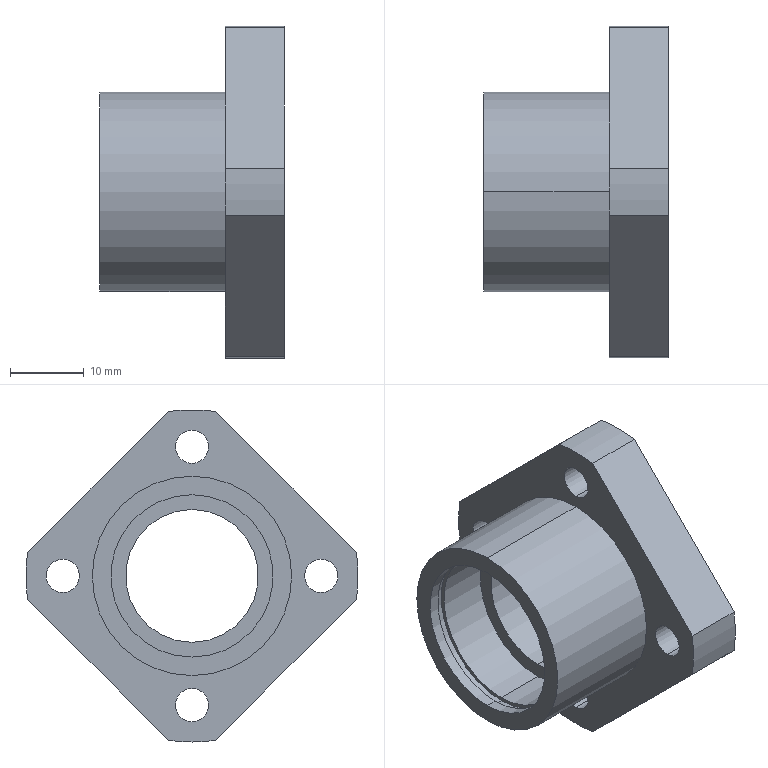Part | SolidWorks | features BaseBody 1 | 1 solid | 54 faces | box 25 x 45 x 45 mm | volume 9867 mm3 | cylinder 37 | plane 17 | commonest cylinder face diameters 4.5 x8 8 x8 22 x8 45 x5 23 x4 18 x2
STEP:
#1=CARTESIAN_POINT('',(-8.,17.5,-2.25));
#2=VERTEX_POINT('',#1);
#3=CARTESIAN_POINT('',(-8.,17.5,2.25));
#4=VERTEX_POINT('',#3);
#5=CARTESIAN_POINT('',(-8.,17.5,0.));
#6=DIRECTION('',(-1.,0.,0.));
#7=DIRECTION('',(0.,0.,-1.));
#8=AXIS2_PLACEMENT_3D('',#5,#6,#7);
#9=CIRCLE('',#8,2.25);
#10=EDGE_CURVE('',#2,#4,#9,.T.);
#11=ORIENTED_EDGE('',*,*,#10,.F.);
#12=CARTESIAN_POINT('',(-8.,17.5,0.));
#13=DIRECTION('',(-1.,0.,0.));
#14=DIRECTION('',(0.,0.,-1.));
#15=AXIS2_PLACEMENT_3D('',#12,#13,#14);
#16=CIRCLE('',#15,2.25);
#17=EDGE_CURVE('',#4,#2,#16,.T.);
#18=ORIENTED_EDGE('',*,*,#17,.F.);
#19=EDGE_LOOP('',(#11,#18));
#20=FACE_BOUND('',#19,.T.);
#21=CARTESIAN_POINT('',(-8.,0.,15.25));
#22=VERTEX_POINT('',#21);
#23=CARTESIAN_POINT('',(-8.,0.,19.75));
#24=VERTEX_POINT('',#23);
#25=CARTESIAN_POINT('',(-8.,0.,17.5));
#26=DIRECTION('',(1.,0.,0.));
#27=DIRECTION('',(0.,0.,-1.));
#28=AXIS2_PLACEMENT_3D('',#25,#26,#27);
#29=CIRCLE('',#28,2.25);
#30=EDGE_CURVE('',#22,#24,#29,.T.);
#31=ORIENTED_EDGE('',*,*,#30,.T.);
#32=CARTESIAN_POINT('',(-8.,0.,17.5));
#33=DIRECTION('',(1.,0.,0.));
#34=DIRECTION('',(0.,0.,-1.));
#35=AXIS2_PLACEMENT_3D('',#32,#33,#34);
#36=CIRCLE('',#35,2.25);
#37=EDGE_CURVE('',#24,#22,#36,.T.);
#38=ORIENTED_EDGE('',*,*,#37,.T.);
#39=EDGE_LOOP('',(#31,#38));
#40=FACE_BOUND('',#39,.T.);
#41=CARTESIAN_POINT('',(-8.,-17.5,-2.25));
#42=VERTEX_POINT('',#41);
#43=CARTESIAN_POINT('',(-8.,-17.5,2.25));
#44=VERTEX_POINT('',#43);
#45=CARTESIAN_POINT('',(-8.,-17.5,0.));
#46=DIRECTION('',(1.,0.,0.));
#47=DIRECTION('',(0.,0.,-1.));
#48=AXIS2_PLACEMENT_3D('',#45,#46,#47);
#49=CIRCLE('',#48,2.25);
#50=EDGE_CURVE('',#42,#44,#49,.T.);
#51=ORIENTED_EDGE('',*,*,#50,.T.);
#52=CARTESIAN_POINT('',(-8.,-17.5,0.));
#53=DIRECTION('',(1.,0.,0.));
#54=DIRECTION('',(0.,0.,-1.));
#55=AXIS2_PLACEMENT_3D('',#52,#53,#54);
#56=CIRCLE('',#55,2.25);
#57=EDGE_CURVE('',#44,#42,#56,.T.);
#58=ORIENTED_EDGE('',*,*,#57,.T.);
#59=EDGE_LOOP('',(#51,#58));
#60=FACE_BOUND('',#59,.T.);
#61=CARTESIAN_POINT('',(-8.,0.,-19.75));
#62=VERTEX_POINT('',#61);
#63=CARTESIAN_POINT('',(-8.,0.,-15.25));
#64=VERTEX_POINT('',#63);
#65=CARTESIAN_POINT('',(-8.,0.,-17.5));
#66=DIRECTION('',(1.,0.,0.));
#67=DIRECTION('',(0.,0.,-1.));
#68=AXIS2_PLACEMENT_3D('',#65,#66,#67);
#69=CIRCLE('',#68,2.25);
#70=EDGE_CURVE('',#62,#64,#69,.T.);
#71=ORIENTED_EDGE('',*,*,#70,.T.);
#72=CARTESIAN_POINT('',(-8.,0.,-17.5));
#73=DIRECTION('',(1.,0.,0.));
#74=DIRECTION('',(0.,0.,-1.));
#75=AXIS2_PLACEMENT_3D('',#72,#73,#74);
#76=CIRCLE('',#75,2.25);
#77=EDGE_CURVE('',#64,#62,#76,.T.);
#78=ORIENTED_EDGE('',*,*,#77,.T.);
#79=EDGE_LOOP('',(#71,#78));
#80=FACE_BOUND('',#79,.T.);
#81=CARTESIAN_POINT('',(-8.,0.,-13.5));
#82=VERTEX_POINT('',#81);
#83=CARTESIAN_POINT('',(-8.,0.,13.5));
#84=VERTEX_POINT('',#83);
#85=CARTESIAN_POINT('',(-8.,0.,0.));
#86=DIRECTION('',(1.,0.,0.));
#87=DIRECTION('',(0.,0.,-1.));
#88=AXIS2_PLACEMENT_3D('',#85,#86,#87);
#89=CIRCLE('',#88,13.5);
#90=EDGE_CURVE('',#82,#84,#89,.T.);
#91=ORIENTED_EDGE('',*,*,#90,.T.);
#92=CARTESIAN_POINT('',(-8.,0.,0.));
#93=DIRECTION('',(1.,0.,0.));
#94=DIRECTION('',(0.,0.,-1.));
#95=AXIS2_PLACEMENT_3D('',#92,#93,#94);
#96=CIRCLE('',#95,13.5);
#97=EDGE_CURVE('',#84,#82,#96,.T.);
#98=ORIENTED_EDGE('',*,*,#97,.T.);
#99=EDGE_LOOP('',(#91,#98));
#100=FACE_BOUND('',#99,.T.);
#101=CARTESIAN_POINT('',(-8.,22.274,-3.182));
#102=VERTEX_POINT('',#101);
#103=CARTESIAN_POINT('',(-8.,22.274,3.182));
#104=VERTEX_POINT('',#103);
#105=CARTESIAN_POINT('',(-8.,0.,0.));
#106=DIRECTION('',(1.,0.,0.));
#107=DIRECTION('',(0.,0.,-1.));
#108=AXIS2_PLACEMENT_3D('',#105,#106,#107);
#109=CIRCLE('',#108,22.5);
#110=EDGE_CURVE('',#102,#104,#109,.T.);
#111=ORIENTED_EDGE('',*,*,#110,.F.);
#112=CARTESIAN_POINT('',(-8.,3.182,-22.274));
#113=VERTEX_POINT('',#112);
#114=CARTESIAN_POINT('',(-8.,0.,-25.456));
#115=DIRECTION('',(0.,0.7071,0.7071));
#116=VECTOR('',#115,1000.);
#117=LINE('',#114,#116);
#118=EDGE_CURVE('',#113,#102,#117,.T.);
#119=ORIENTED_EDGE('',*,*,#118,.F.);
#120=CARTESIAN_POINT('',(-8.,0.,-22.5));
#121=VERTEX_POINT('',#120);
#122=CARTESIAN_POINT('',(-8.,0.,0.));
#123=DIRECTION('',(1.,0.,0.));
#124=DIRECTION('',(0.,0.,-1.));
#125=AXIS2_PLACEMENT_3D('',#122,#123,#124);
#126=CIRCLE('',#125,22.5);
#127=EDGE_CURVE('',#121,#113,#126,.T.);
#128=ORIENTED_EDGE('',*,*,#127,.F.);
#129=CARTESIAN_POINT('',(-8.,-3.182,-22.274));
#130=VERTEX_POINT('',#129);
#131=CARTESIAN_POINT('',(-8.,0.,0.));
#132=DIRECTION('',(1.,0.,0.));
#133=DIRECTION('',(0.,0.,-1.));
#134=AXIS2_PLACEMENT_3D('',#131,#132,#133);
#135=CIRCLE('',#134,22.5);
#136=EDGE_CURVE('',#130,#121,#135,.T.);
#137=ORIENTED_EDGE('',*,*,#136,.F.);
#138=CARTESIAN_POINT('',(-8.,-22.274,-3.182));
#139=VERTEX_POINT('',#138);
#140=CARTESIAN_POINT('',(-8.,-25.456,0.));
#141=DIRECTION('',(0.,0.7071,-0.7071));
#142=VECTOR('',#141,1000.);
#143=LINE('',#140,#142);
#144=EDGE_CURVE('',#139,#130,#143,.T.);
#145=ORIENTED_EDGE('',*,*,#144,.F.);
#146=CARTESIAN_POINT('',(-8.,-22.274,3.182));
#147=VERTEX_POINT('',#146);
#148=CARTESIAN_POINT('',(-8.,0.,0.));
#149=DIRECTION('',(1.,0.,0.));
#150=DIRECTION('',(0.,0.,-1.));
#151=AXIS2_PLACEMENT_3D('',#148,#149,#150);
#152=CIRCLE('',#151,22.5);
#153=EDGE_CURVE('',#147,#139,#152,.T.);
#154=ORIENTED_EDGE('',*,*,#153,.F.);
#155=CARTESIAN_POINT('',(-8.,-3.182,22.274));
#156=VERTEX_POINT('',#155);
#157=CARTESIAN_POINT('',(-8.,0.,25.456));
#158=DIRECTION('',(0.,-0.7071,-0.7071));
#159=VECTOR('',#158,1000.);
#160=LINE('',#157,#159);
#161=EDGE_CURVE('',#156,#147,#160,.T.);
#162=ORIENTED_EDGE('',*,*,#161,.F.);
#163=CARTESIAN_POINT('',(-8.,3.182,22.274));
#164=VERTEX_POINT('',#163);
#165=CARTESIAN_POINT('',(-8.,0.,0.));
#166=DIRECTION('',(1.,0.,0.));
#167=DIRECTION('',(0.,0.,-1.));
#168=AXIS2_PLACEMENT_3D('',#165,#166,#167);
#169=CIRCLE('',#168,22.5);
#170=EDGE_CURVE('',#164,#156,#169,.T.);
#171=ORIENTED_EDGE('',*,*,#170,.F.);
#172=CARTESIAN_POINT('',(-8.,25.456,0.));
#173=DIRECTION('',(0.,-0.7071,0.7071));
#174=VECTOR('',#173,1000.);
#175=LINE('',#172,#174);
#176=EDGE_CURVE('',#104,#164,#175,.T.);
#177=ORIENTED_EDGE('',*,*,#176,.F.);
#178=EDGE_LOOP('',(#111,#119,#128,#137,#145,#154,#162,#171,#177));
#179=FACE_OUTER_BOUND('',#178,.T.);
#180=CARTESIAN_POINT('',(-8.,13.5,0.));
#181=DIRECTION('',(1.,0.,0.));
#182=DIRECTION('',(0.,1.,0.));
#183=AXIS2_PLACEMENT_3D('',#180,#181,#182);
#184=PLANE('',#183);
#185=ADVANCED_FACE('',(#20,#40,#60,#80,#100,#179),#184,.F.);
#186=CARTESIAN_POINT('',(0.,3.182,22.274));
#187=VERTEX_POINT('',#186);
#188=CARTESIAN_POINT('',(0.,3.182,22.274));
#189=DIRECTION('',(1.,0.,0.));
#190=VECTOR('',#189,1000.);
#191=LINE('',#188,#190);
#192=EDGE_CURVE('',#164,#187,#191,.T.);
#193=ORIENTED_EDGE('',*,*,#192,.F.);
#194=ORIENTED_EDGE('',*,*,#170,.T.);
#195=CARTESIAN_POINT('',(0.,-3.182,22.274));
#196=VERTEX_POINT('',#195);
#197=CARTESIAN_POINT('',(0.,-3.182,22.274));
#198=DIRECTION('',(-1.,0.,0.));
#199=VECTOR('',#198,1000.);
#200=LINE('',#197,#199);
#201=EDGE_CURVE('',#196,#156,#200,.T.);
#202=ORIENTED_EDGE('',*,*,#201,.F.);
#203=CARTESIAN_POINT('',(0.,0.,0.));
#204=DIRECTION('',(1.,0.,0.));
#205=DIRECTION('',(0.,0.,-1.));
#206=AXIS2_PLACEMENT_3D('',#203,#204,#205);
#207=CIRCLE('',#206,22.5);
#208=EDGE_CURVE('',#187,#196,#207,.T.);
#209=ORIENTED_EDGE('',*,*,#208,.F.);
#210=EDGE_LOOP('',(#193,#194,#202,#209));
#211=FACE_OUTER_BOUND('',#210,.T.);
#212=CARTESIAN_POINT('',(0.,0.,0.));
#213=DIRECTION('',(1.,0.,0.));
#214=DIRECTION('',(0.,0.,-1.));
#215=AXIS2_PLACEMENT_3D('',#212,#213,#214);
#216=CYLINDRICAL_SURFACE('',#215,22.5);
#217=ADVANCED_FACE('',(#211),#216,.T.);
#218=CARTESIAN_POINT('',(0.,22.274,-3.182));
#219=VERTEX_POINT('',#218);
#220=CARTESIAN_POINT('',(0.,22.274,-3.182));
#221=DIRECTION('',(1.,0.,0.));
#222=VECTOR('',#221,1000.);
#223=LINE('',#220,#222);
#224=EDGE_CURVE('',#102,#219,#223,.T.);
#225=ORIENTED_EDGE('',*,*,#224,.F.);
#226=ORIENTED_EDGE('',*,*,#110,.T.);
#227=CARTESIAN_POINT('',(0.,22.274,3.182));
#228=VERTEX_POINT('',#227);
#229=CARTESIAN_POINT('',(0.,22.274,3.182));
#230=DIRECTION('',(-1.,0.,0.));
#231=VECTOR('',#230,1000.);
#232=LINE('',#229,#231);
#233=EDGE_CURVE('',#228,#104,#232,.T.);
#234=ORIENTED_EDGE('',*,*,#233,.F.);
#235=CARTESIAN_POINT('',(0.,0.,0.));
#236=DIRECTION('',(1.,0.,0.));
#237=DIRECTION('',(0.,0.,-1.));
#238=AXIS2_PLACEMENT_3D('',#235,#236,#237);
#239=CIRCLE('',#238,22.5);
#240=EDGE_CURVE('',#219,#228,#239,.T.);
#241=ORIENTED_EDGE('',*,*,#240,.F.);
#242=EDGE_LOOP('',(#225,#226,#234,#241));
#243=FACE_OUTER_BOUND('',#242,.T.);
#244=CARTESIAN_POINT('',(0.,0.,0.));
#245=DIRECTION('',(1.,0.,0.));
#246=DIRECTION('',(0.,0.,-1.));
#247=AXIS2_PLACEMENT_3D('',#244,#245,#246);
#248=CYLINDRICAL_SURFACE('',#247,22.5);
#249=ADVANCED_FACE('',(#243),#248,.T.);
#250=CARTESIAN_POINT('',(0.,0.,-22.5));
#251=VERTEX_POINT('',#250);
#252=CARTESIAN_POINT('',(0.,0.,-22.5));
#253=DIRECTION('',(1.,0.,0.));
#254=VECTOR('',#253,1000.);
#255=LINE('',#252,#254);
#256=EDGE_CURVE('',#121,#251,#255,.T.);
#257=ORIENTED_EDGE('',*,*,#256,.F.);
#258=ORIENTED_EDGE('',*,*,#127,.T.);
#259=CARTESIAN_POINT('',(0.,3.182,-22.274));
#260=VERTEX_POINT('',#259);
#261=CARTESIAN_POINT('',(0.,3.182,-22.274));
#262=DIRECTION('',(-1.,0.,0.));
#263=VECTOR('',#262,1000.);
#264=LINE('',#261,#263);
#265=EDGE_CURVE('',#260,#113,#264,.T.);
#266=ORIENTED_EDGE('',*,*,#265,.F.);
#267=CARTESIAN_POINT('',(0.,0.,0.));
#268=DIRECTION('',(1.,0.,0.));
#269=DIRECTION('',(0.,0.,-1.));
#270=AXIS2_PLACEMENT_3D('',#267,#268,#269);
#271=CIRCLE('',#270,22.5);
#272=EDGE_CURVE('',#251,#260,#271,.T.);
#273=ORIENTED_EDGE('',*,*,#272,.F.);
#274=EDGE_LOOP('',(#257,#258,#266,#273));
#275=FACE_OUTER_BOUND('',#274,.T.);
#276=CARTESIAN_POINT('',(0.,0.,0.));
#277=DIRECTION('',(1.,0.,0.));
#278=DIRECTION('',(0.,0.,-1.));
#279=AXIS2_PLACEMENT_3D('',#276,#277,#278);
#280=CYLINDRICAL_SURFACE('',#279,22.5);
#281=ADVANCED_FACE('',(#275),#280,.T.);
#282=CARTESIAN_POINT('',(0.,-22.274,-3.182));
#283=VERTEX_POINT('',#282);
#284=CARTESIAN_POINT('',(0.,-22.274,-3.182));
#285=DIRECTION('',(-1.,0.,0.));
#286=VECTOR('',#285,1000.);
#287=LINE('',#284,#286);
#288=EDGE_CURVE('',#283,#139,#287,.T.);
#289=ORIENTED_EDGE('',*,*,#288,.F.);
#290=CARTESIAN_POINT('',(0.,-22.274,3.182));
#291=VERTEX_POINT('',#290);
#292=CARTESIAN_POINT('',(0.,0.,0.));
#293=DIRECTION('',(1.,0.,0.));
#294=DIRECTION('',(0.,0.,-1.));
#295=AXIS2_PLACEMENT_3D('',#292,#293,#294);
#296=CIRCLE('',#295,22.5);
#297=EDGE_CURVE('',#291,#283,#296,.T.);
#298=ORIENTED_EDGE('',*,*,#297,.F.);
#299=CARTESIAN_POINT('',(0.,-22.274,3.182));
#300=DIRECTION('',(1.,0.,0.));
#301=VECTOR('',#300,1000.);
#302=LINE('',#299,#301);
#303=EDGE_CURVE('',#147,#291,#302,.T.);
#304=ORIENTED_EDGE('',*,*,#303,.F.);
#305=ORIENTED_EDGE('',*,*,#153,.T.);
#306=EDGE_LOOP('',(#289,#298,#304,#305));
#307=FACE_OUTER_BOUND('',#306,.T.);
#308=CARTESIAN_POINT('',(0.,0.,0.));
#309=DIRECTION('',(1.,0.,0.));
#310=DIRECTION('',(0.,0.,-1.));
#311=AXIS2_PLACEMENT_3D('',#308,#309,#310);
#312=CYLINDRICAL_SURFACE('',#311,22.5);
#313=ADVANCED_FACE('',(#307),#312,.T.);
#314=CARTESIAN_POINT('',(0.,0.,-11.));
#315=VERTEX_POINT('',#314);
#316=CARTESIAN_POINT('',(0.,0.,11.));
#317=VERTEX_POINT('',#316);
#318=CARTESIAN_POINT('',(0.,0.,0.));
#319=DIRECTION('',(1.,0.,0.));
#320=DIRECTION('',(0.,0.,-1.));
#321=AXIS2_PLACEMENT_3D('',#318,#319,#320);
#322=CIRCLE('',#321,11.);
#323=EDGE_CURVE('',#315,#317,#322,.T.);
#324=ORIENTED_EDGE('',*,*,#323,.F.);
#325=CARTESIAN_POINT('',(0.,0.,0.));
#326=DIRECTION('',(1.,0.,0.));
#327=DIRECTION('',(0.,0.,-1.));
#328=AXIS2_PLACEMENT_3D('',#325,#326,#327);
#329=CIRCLE('',#328,11.);
#330=EDGE_CURVE('',#317,#315,#329,.T.);
#331=ORIENTED_EDGE('',*,*,#330,.F.);
#332=EDGE_LOOP('',(#324,#331));
#333=FACE_BOUND('',#332,.T.);
#334=CARTESIAN_POINT('',(0.,17.5,-4.));
#335=VERTEX_POINT('',#334);
#336=CARTESIAN_POINT('',(0.,17.5,4.));
#337=VERTEX_POINT('',#336);
#338=CARTESIAN_POINT('',(0.,17.5,0.));
#339=DIRECTION('',(1.,0.,0.));
#340=DIRECTION('',(0.,0.,1.));
#341=AXIS2_PLACEMENT_3D('',#338,#339,#340);
#342=CIRCLE('',#341,4.);
#343=EDGE_CURVE('',#335,#337,#342,.T.);
#344=ORIENTED_EDGE('',*,*,#343,.F.);
#345=CARTESIAN_POINT('',(0.,17.5,0.));
#346=DIRECTION('',(1.,0.,0.));
#347=DIRECTION('',(0.,0.,1.));
#348=AXIS2_PLACEMENT_3D('',#345,#346,#347);
#349=CIRCLE('',#348,4.);
#350=EDGE_CURVE('',#337,#335,#349,.T.);
#351=ORIENTED_EDGE('',*,*,#350,.F.);
#352=EDGE_LOOP('',(#344,#351));
#353=FACE_BOUND('',#352,.T.);
#354=CARTESIAN_POINT('',(0.,0.,13.5));
#355=VERTEX_POINT('',#354);
#356=CARTESIAN_POINT('',(0.,0.,21.5));
#357=VERTEX_POINT('',#356);
#358=CARTESIAN_POINT('',(0.,0.,17.5));
#359=DIRECTION('',(1.,0.,0.));
#360=DIRECTION('',(0.,0.,-1.));
#361=AXIS2_PLACEMENT_3D('',#358,#359,#360);
#362=CIRCLE('',#361,4.);
#363=EDGE_CURVE('',#355,#357,#362,.T.);
#364=ORIENTED_EDGE('',*,*,#363,.F.);
#365=CARTESIAN_POINT('',(0.,0.,17.5));
#366=DIRECTION('',(1.,0.,0.));
#367=DIRECTION('',(0.,0.,-1.));
#368=AXIS2_PLACEMENT_3D('',#365,#366,#367);
#369=CIRCLE('',#368,4.);
#370=EDGE_CURVE('',#357,#355,#369,.T.);
#371=ORIENTED_EDGE('',*,*,#370,.F.);
#372=EDGE_LOOP('',(#364,#371));
#373=FACE_BOUND('',#372,.T.);
#374=CARTESIAN_POINT('',(0.,-17.5,-4.));
#375=VERTEX_POINT('',#374);
#376=CARTESIAN_POINT('',(0.,-17.5,4.));
#377=VERTEX_POINT('',#376);
#378=CARTESIAN_POINT('',(0.,-17.5,0.));
#379=DIRECTION('',(1.,0.,0.));
#380=DIRECTION('',(0.,0.,-1.));
#381=AXIS2_PLACEMENT_3D('',#378,#379,#380);
#382=CIRCLE('',#381,4.);
#383=EDGE_CURVE('',#375,#377,#382,.T.);
#384=ORIENTED_EDGE('',*,*,#383,.F.);
#385=CARTESIAN_POINT('',(0.,-17.5,0.));
#386=DIRECTION('',(1.,0.,0.));
#387=DIRECTION('',(0.,0.,-1.));
#388=AXIS2_PLACEMENT_3D('',#385,#386,#387);
#389=CIRCLE('',#388,4.);
#390=EDGE_CURVE('',#377,#375,#389,.T.);
#391=ORIENTED_EDGE('',*,*,#390,.F.);
#392=EDGE_LOOP('',(#384,#391));
#393=FACE_BOUND('',#392,.T.);
#394=CARTESIAN_POINT('',(0.,0.,-21.5));
#395=VERTEX_POINT('',#394);
#396=CARTESIAN_POINT('',(0.,0.,-13.5));
#397=VERTEX_POINT('',#396);
#398=CARTESIAN_POINT('',(0.,0.,-17.5));
#399=DIRECTION('',(1.,0.,0.));
#400=DIRECTION('',(0.,0.,-1.));
#401=AXIS2_PLACEMENT_3D('',#398,#399,#400);
#402=CIRCLE('',#401,4.);
#403=EDGE_CURVE('',#395,#397,#402,.T.);
#404=ORIENTED_EDGE('',*,*,#403,.F.);
#405=CARTESIAN_POINT('',(0.,0.,-17.5));
#406=DIRECTION('',(1.,0.,0.));
#407=DIRECTION('',(0.,0.,-1.));
#408=AXIS2_PLACEMENT_3D('',#405,#406,#407);
#409=CIRCLE('',#408,4.);
#410=EDGE_CURVE('',#397,#395,#409,.T.);
#411=ORIENTED_EDGE('',*,*,#410,.F.);
#412=EDGE_LOOP('',(#404,#411));
#413=FACE_BOUND('',#412,.T.);
#414=CARTESIAN_POINT('',(0.,23.978,-1.478));
#415=DIRECTION('',(0.,-0.7071,-0.7071));
#416=VECTOR('',#415,1000.);
#417=LINE('',#414,#416);
#418=EDGE_CURVE('',#219,#260,#417,.T.);
#419=ORIENTED_EDGE('',*,*,#418,.F.);
#420=ORIENTED_EDGE('',*,*,#240,.T.);
#421=CARTESIAN_POINT('',(0.,23.978,1.478));
#422=DIRECTION('',(0.,0.7071,-0.7071));
#423=VECTOR('',#422,1000.);
#424=LINE('',#421,#423);
#425=EDGE_CURVE('',#187,#228,#424,.T.);
#426=ORIENTED_EDGE('',*,*,#425,.F.);
#427=ORIENTED_EDGE('',*,*,#208,.T.);
#428=CARTESIAN_POINT('',(0.,-1.478,23.978));
#429=DIRECTION('',(0.,0.7071,0.7071));
#430=VECTOR('',#429,1000.);
#431=LINE('',#428,#430);
#432=EDGE_CURVE('',#291,#196,#431,.T.);
#433=ORIENTED_EDGE('',*,*,#432,.F.);
#434=ORIENTED_EDGE('',*,*,#297,.T.);
#435=CARTESIAN_POINT('',(0.,-3.182,-22.274));
#436=VERTEX_POINT('',#435);
#437=CARTESIAN_POINT('',(0.,-1.478,-23.978));
#438=DIRECTION('',(0.,-0.7071,0.7071));
#439=VECTOR('',#438,1000.);
#440=LINE('',#437,#439);
#441=EDGE_CURVE('',#436,#283,#440,.T.);
#442=ORIENTED_EDGE('',*,*,#441,.F.);
#443=CARTESIAN_POINT('',(0.,0.,0.));
#444=DIRECTION('',(1.,0.,0.));
#445=DIRECTION('',(0.,0.,-1.));
#446=AXIS2_PLACEMENT_3D('',#443,#444,#445);
#447=CIRCLE('',#446,22.5);
#448=EDGE_CURVE('',#436,#251,#447,.T.);
#449=ORIENTED_EDGE('',*,*,#448,.T.);
#450=ORIENTED_EDGE('',*,*,#272,.T.);
#451=EDGE_LOOP('',(#419,#420,#426,#427,#433,#434,#442,#449,#450));
#452=FACE_OUTER_BOUND('',#451,.T.);
#453=CARTESIAN_POINT('',(0.,22.5,0.));
#454=DIRECTION('',(-1.,0.,0.));
#455=DIRECTION('',(0.,0.,1.));
#456=AXIS2_PLACEMENT_3D('',#453,#454,#455);
#457=PLANE('',#456);
#458=ADVANCED_FACE('',(#333,#353,#373,#393,#413,#452),#457,.F.);
#459=CARTESIAN_POINT('',(-25.,0.,-11.));
#460=VERTEX_POINT('',#459);
#461=CARTESIAN_POINT('',(-25.,0.,11.));
#462=VERTEX_POINT('',#461);
#463=CARTESIAN_POINT('',(-25.,0.,0.));
#464=DIRECTION('',(1.,0.,0.));
#465=DIRECTION('',(0.,0.,-1.));
#466=AXIS2_PLACEMENT_3D('',#463,#464,#465);
#467=CIRCLE('',#466,11.);
#468=EDGE_CURVE('',#460,#462,#467,.T.);
#469=ORIENTED_EDGE('',*,*,#468,.T.);
#470=CARTESIAN_POINT('',(-25.,0.,0.));
#471=DIRECTION('',(1.,0.,0.));
#472=DIRECTION('',(0.,0.,-1.));
#473=AXIS2_PLACEMENT_3D('',#470,#471,#472);
#474=CIRCLE('',#473,11.);
#475=EDGE_CURVE('',#462,#460,#474,.T.);
#476=ORIENTED_EDGE('',*,*,#475,.T.);
#477=EDGE_LOOP('',(#469,#476));
#478=FACE_BOUND('',#477,.T.);
#479=CARTESIAN_POINT('',(-25.,0.,-13.5));
#480=VERTEX_POINT('',#479);
#481=CARTESIAN_POINT('',(-25.,0.,13.5));
#482=VERTEX_POINT('',#481);
#483=CARTESIAN_POINT('',(-25.,0.,0.));
#484=DIRECTION('',(1.,0.,0.));
#485=DIRECTION('',(0.,0.,-1.));
#486=AXIS2_PLACEMENT_3D('',#483,#484,#485);
#487=CIRCLE('',#486,13.5);
#488=EDGE_CURVE('',#480,#482,#487,.T.);
#489=ORIENTED_EDGE('',*,*,#488,.F.);
#490=CARTESIAN_POINT('',(-25.,0.,0.));
#491=DIRECTION('',(1.,0.,0.));
#492=DIRECTION('',(0.,0.,-1.));
#493=AXIS2_PLACEMENT_3D('',#490,#491,#492);
#494=CIRCLE('',#493,13.5);
#495=EDGE_CURVE('',#482,#480,#494,.T.);
#496=ORIENTED_EDGE('',*,*,#495,.F.);
#497=EDGE_LOOP('',(#489,#496));
#498=FACE_OUTER_BOUND('',#497,.T.);
#499=CARTESIAN_POINT('',(-25.,0.,0.));
#500=DIRECTION('',(1.,0.,0.));
#501=DIRECTION('',(0.,1.,0.));
#502=AXIS2_PLACEMENT_3D('',#499,#500,#501);
#503=PLANE('',#502);
#504=ADVANCED_FACE('',(#478,#498),#503,.F.);
#505=CARTESIAN_POINT('',(0.,0.,13.5));
#506=DIRECTION('',(1.,0.,0.));
#507=VECTOR('',#506,1000.);
#508=LINE('',#505,#507);
#509=EDGE_CURVE('',#482,#84,#508,.T.);
#510=ORIENTED_EDGE('',*,*,#509,.F.);
#511=ORIENTED_EDGE('',*,*,#495,.T.);
#512=CARTESIAN_POINT('',(0.,0.,-13.5));
#513=DIRECTION('',(1.,0.,0.));
#514=VECTOR('',#513,1000.);
#515=LINE('',#512,#514);
#516=EDGE_CURVE('',#480,#82,#515,.T.);
#517=ORIENTED_EDGE('',*,*,#516,.T.);
#518=ORIENTED_EDGE('',*,*,#97,.F.);
#519=EDGE_LOOP('',(#510,#511,#517,#518));
#520=FACE_OUTER_BOUND('',#519,.T.);
#521=CARTESIAN_POINT('',(0.,0.,0.));
#522=DIRECTION('',(1.,0.,0.));
#523=DIRECTION('',(0.,0.,-1.));
#524=AXIS2_PLACEMENT_3D('',#521,#522,#523);
#525=CYLINDRICAL_SURFACE('',#524,13.5);
#526=ADVANCED_FACE('',(#520),#525,.T.);
#527=CARTESIAN_POINT('',(-23.5,0.,11.));
#528=VERTEX_POINT('',#527);
#529=CARTESIAN_POINT('',(0.,0.,11.));
#530=DIRECTION('',(1.,0.,0.));
#531=VECTOR('',#530,1000.);
#532=LINE('',#529,#531);
#533=EDGE_CURVE('',#462,#528,#532,.T.);
#534=ORIENTED_EDGE('',*,*,#533,.F.);
#535=ORIENTED_EDGE('',*,*,#468,.F.);
#536=CARTESIAN_POINT('',(-23.5,0.,-11.));
#537=VERTEX_POINT('',#536);
#538=CARTESIAN_POINT('',(0.,0.,-11.));
#539=DIRECTION('',(1.,0.,0.));
#540=VECTOR('',#539,1000.);
#541=LINE('',#538,#540);
#542=EDGE_CURVE('',#460,#537,#541,.T.);
#543=ORIENTED_EDGE('',*,*,#542,.T.);
#544=CARTESIAN_POINT('',(-23.5,0.,0.));
#545=DIRECTION('',(1.,0.,0.));
#546=DIRECTION('',(0.,0.,-1.));
#547=AXIS2_PLACEMENT_3D('',#544,#545,#546);
#548=CIRCLE('',#547,11.);
#549=EDGE_CURVE('',#537,#528,#548,.T.);
#550=ORIENTED_EDGE('',*,*,#549,.T.);
#551=EDGE_LOOP('',(#534,#535,#543,#550));
#552=FACE_OUTER_BOUND('',#551,.T.);
#553=CARTESIAN_POINT('',(0.,0.,0.));
#554=DIRECTION('',(1.,0.,0.));
#555=DIRECTION('',(0.,0.,-1.));
#556=AXIS2_PLACEMENT_3D('',#553,#554,#555);
#557=CYLINDRICAL_SURFACE('',#556,11.);
#558=ADVANCED_FACE('',(#552),#557,.F.);
#559=ORIENTED_EDGE('',*,*,#549,.F.);
#560=CARTESIAN_POINT('',(-23.5,0.,0.));
#561=DIRECTION('',(1.,0.,0.));
#562=DIRECTION('',(0.,0.,-1.));
#563=AXIS2_PLACEMENT_3D('',#560,#561,#562);
#564=CIRCLE('',#563,11.);
#565=EDGE_CURVE('',#528,#537,#564,.T.);
#566=ORIENTED_EDGE('',*,*,#565,.F.);
#567=EDGE_LOOP('',(#559,#566));
#568=FACE_BOUND('',#567,.T.);
#569=CARTESIAN_POINT('',(-23.5,0.,-11.5));
#570=VERTEX_POINT('',#569);
#571=CARTESIAN_POINT('',(-23.5,0.,11.5));
#572=VERTEX_POINT('',#571);
#573=CARTESIAN_POINT('',(-23.5,0.,0.));
#574=DIRECTION('',(1.,0.,0.));
#575=DIRECTION('',(0.,0.,-1.));
#576=AXIS2_PLACEMENT_3D('',#573,#574,#575);
#577=CIRCLE('',#576,11.5);
#578=EDGE_CURVE('',#570,#572,#577,.T.);
#579=ORIENTED_EDGE('',*,*,#578,.T.);
#580=CARTESIAN_POINT('',(-23.5,0.,0.));
#581=DIRECTION('',(1.,0.,0.));
#582=DIRECTION('',(0.,0.,-1.));
#583=AXIS2_PLACEMENT_3D('',#580,#581,#582);
#584=CIRCLE('',#583,11.5);
#585=EDGE_CURVE('',#572,#570,#584,.T.);
#586=ORIENTED_EDGE('',*,*,#585,.T.);
#587=EDGE_LOOP('',(#579,#586));
#588=FACE_OUTER_BOUND('',#587,.T.);
#589=CARTESIAN_POINT('',(-23.5,11.,0.));
#590=DIRECTION('',(1.,0.,0.));
#591=DIRECTION('',(0.,1.,0.));
#592=AXIS2_PLACEMENT_3D('',#589,#590,#591);
#593=PLANE('',#592);
#594=ADVANCED_FACE('',(#568,#588),#593,.T.);
#595=CARTESIAN_POINT('',(-22.35,0.,11.5));
#596=VERTEX_POINT('',#595);
#597=CARTESIAN_POINT('',(0.,0.,11.5));
#598=DIRECTION('',(1.,0.,0.));
#599=VECTOR('',#598,1000.);
#600=LINE('',#597,#599);
#601=EDGE_CURVE('',#572,#596,#600,.T.);
#602=ORIENTED_EDGE('',*,*,#601,.F.);
#603=ORIENTED_EDGE('',*,*,#578,.F.);
#604=CARTESIAN_POINT('',(-22.35,0.,-11.5));
#605=VERTEX_POINT('',#604);
#606=CARTESIAN_POINT('',(0.,0.,-11.5));
#607=DIRECTION('',(1.,0.,0.));
#608=VECTOR('',#607,1000.);
#609=LINE('',#606,#608);
#610=EDGE_CURVE('',#570,#605,#609,.T.);
#611=ORIENTED_EDGE('',*,*,#610,.T.);
#612=CARTESIAN_POINT('',(-22.35,0.,0.));
#613=DIRECTION('',(1.,0.,0.));
#614=DIRECTION('',(0.,0.,-1.));
#615=AXIS2_PLACEMENT_3D('',#612,#613,#614);
#616=CIRCLE('',#615,11.5);
#617=EDGE_CURVE('',#605,#596,#616,.T.);
#618=ORIENTED_EDGE('',*,*,#617,.T.);
#619=EDGE_LOOP('',(#602,#603,#611,#618));
#620=FACE_OUTER_BOUND('',#619,.T.);
#621=CARTESIAN_POINT('',(0.,0.,0.));
#622=DIRECTION('',(1.,0.,0.));
#623=DIRECTION('',(0.,0.,-1.));
#624=AXIS2_PLACEMENT_3D('',#621,#622,#623);
#625=CYLINDRICAL_SURFACE('',#624,11.5);
#626=ADVANCED_FACE('',(#620),#625,.F.);
#627=CARTESIAN_POINT('',(-22.35,0.,-11.));
#628=VERTEX_POINT('',#627);
#629=CARTESIAN_POINT('',(-22.35,0.,11.));
#630=VERTEX_POINT('',#629);
#631=CARTESIAN_POINT('',(-22.35,0.,0.));
#632=DIRECTION('',(1.,0.,0.));
#633=DIRECTION('',(0.,0.,-1.));
#634=AXIS2_PLACEMENT_3D('',#631,#632,#633);
#635=CIRCLE('',#634,11.);
#636=EDGE_CURVE('',#628,#630,#635,.T.);
#637=ORIENTED_EDGE('',*,*,#636,.T.);
#638=CARTESIAN_POINT('',(-22.35,0.,0.));
#639=DIRECTION('',(1.,0.,0.));
#640=DIRECTION('',(0.,0.,-1.));
#641=AXIS2_PLACEMENT_3D('',#638,#639,#640);
#642=CIRCLE('',#641,11.);
#643=EDGE_CURVE('',#630,#628,#642,.T.);
#644=ORIENTED_EDGE('',*,*,#643,.T.);
#645=EDGE_LOOP('',(#637,#644));
#646=FACE_BOUND('',#645,.T.);
#647=ORIENTED_EDGE('',*,*,#617,.F.);
#648=CARTESIAN_POINT('',(-22.35,0.,0.));
#649=DIRECTION('',(1.,0.,0.));
#650=DIRECTION('',(0.,0.,-1.));
#651=AXIS2_PLACEMENT_3D('',#648,#649,#650);
#652=CIRCLE('',#651,11.5);
#653=EDGE_CURVE('',#596,#605,#652,.T.);
#654=ORIENTED_EDGE('',*,*,#653,.F.);
#655=EDGE_LOOP('',(#647,#654));
#656=FACE_OUTER_BOUND('',#655,.T.);
#657=CARTESIAN_POINT('',(-22.35,11.5,0.));
#658=DIRECTION('',(-1.,0.,0.));
#659=DIRECTION('',(0.,0.,1.));
#660=AXIS2_PLACEMENT_3D('',#657,#658,#659);
#661=PLANE('',#660);
#662=ADVANCED_FACE('',(#646,#656),#661,.T.);
#663=CARTESIAN_POINT('',(-15.35,0.,11.));
#664=VERTEX_POINT('',#663);
#665=CARTESIAN_POINT('',(0.,0.,11.));
#666=DIRECTION('',(1.,0.,0.));
#667=VECTOR('',#666,1000.);
#668=LINE('',#665,#667);
#669=EDGE_CURVE('',#630,#664,#668,.T.);
#670=ORIENTED_EDGE('',*,*,#669,.F.);
#671=ORIENTED_EDGE('',*,*,#636,.F.);
#672=CARTESIAN_POINT('',(-15.35,0.,-11.));
#673=VERTEX_POINT('',#672);
#674=CARTESIAN_POINT('',(0.,0.,-11.));
#675=DIRECTION('',(1.,0.,0.));
#676=VECTOR('',#675,1000.);
#677=LINE('',#674,#676);
#678=EDGE_CURVE('',#628,#673,#677,.T.);
#679=ORIENTED_EDGE('',*,*,#678,.T.);
#680=CARTESIAN_POINT('',(-15.35,0.,0.));
#681=DIRECTION('',(1.,0.,0.));
#682=DIRECTION('',(0.,0.,-1.));
#683=AXIS2_PLACEMENT_3D('',#680,#681,#682);
#684=CIRCLE('',#683,11.);
#685=EDGE_CURVE('',#673,#664,#684,.T.);
#686=ORIENTED_EDGE('',*,*,#685,.T.);
#687=EDGE_LOOP('',(#670,#671,#679,#686));
#688=FACE_OUTER_BOUND('',#687,.T.);
#689=CARTESIAN_POINT('',(0.,0.,0.));
#690=DIRECTION('',(1.,0.,0.));
#691=DIRECTION('',(0.,0.,-1.));
#692=AXIS2_PLACEMENT_3D('',#689,#690,#691);
#693=CYLINDRICAL_SURFACE('',#692,11.);
#694=ADVANCED_FACE('',(#688),#693,.F.);
#695=CARTESIAN_POINT('',(-15.35,0.,-9.));
#696=VERTEX_POINT('',#695);
#697=CARTESIAN_POINT('',(-15.35,0.,9.));
#698=VERTEX_POINT('',#697);
#699=CARTESIAN_POINT('',(-15.35,0.,0.));
#700=DIRECTION('',(1.,0.,0.));
#701=DIRECTION('',(0.,0.,-1.));
#702=AXIS2_PLACEMENT_3D('',#699,#700,#701);
#703=CIRCLE('',#702,9.);
#704=EDGE_CURVE('',#696,#698,#703,.T.);
#705=ORIENTED_EDGE('',*,*,#704,.T.);
#706=CARTESIAN_POINT('',(-15.35,0.,0.));
#707=DIRECTION('',(1.,0.,0.));
#708=DIRECTION('',(0.,0.,-1.));
#709=AXIS2_PLACEMENT_3D('',#706,#707,#708);
#710=CIRCLE('',#709,9.);
#711=EDGE_CURVE('',#698,#696,#710,.T.);
#712=ORIENTED_EDGE('',*,*,#711,.T.);
#713=EDGE_LOOP('',(#705,#712));
#714=FACE_BOUND('',#713,.T.);
#715=ORIENTED_EDGE('',*,*,#685,.F.);
#716=CARTESIAN_POINT('',(-15.35,0.,0.));
#717=DIRECTION('',(1.,0.,0.));
#718=DIRECTION('',(0.,0.,-1.));
#719=AXIS2_PLACEMENT_3D('',#716,#717,#718);
#720=CIRCLE('',#719,11.);
#721=EDGE_CURVE('',#664,#673,#720,.T.);
#722=ORIENTED_EDGE('',*,*,#721,.F.);
#723=EDGE_LOOP('',(#715,#722));
#724=FACE_OUTER_BOUND('',#723,.T.);
#725=CARTESIAN_POINT('',(-15.35,11.,0.));
#726=DIRECTION('',(-1.,0.,0.));
#727=DIRECTION('',(0.,0.,1.));
#728=AXIS2_PLACEMENT_3D('',#725,#726,#727);
#729=PLANE('',#728);
#730=ADVANCED_FACE('',(#714,#724),#729,.T.);
#731=CARTESIAN_POINT('',(-9.65,0.,9.));
#732=VERTEX_POINT('',#731);
#733=CARTESIAN_POINT('',(0.,0.,9.));
#734=DIRECTION('',(1.,0.,0.));
#735=VECTOR('',#734,1000.);
#736=LINE('',#733,#735);
#737=EDGE_CURVE('',#698,#732,#736,.T.);
#738=ORIENTED_EDGE('',*,*,#737,.F.);
#739=ORIENTED_EDGE('',*,*,#704,.F.);
#740=CARTESIAN_POINT('',(-9.65,0.,-9.));
#741=VERTEX_POINT('',#740);
#742=CARTESIAN_POINT('',(0.,0.,-9.));
#743=DIRECTION('',(1.,0.,0.));
#744=VECTOR('',#743,1000.);
#745=LINE('',#742,#744);
#746=EDGE_CURVE('',#696,#741,#745,.T.);
#747=ORIENTED_EDGE('',*,*,#746,.T.);
#748=CARTESIAN_POINT('',(-9.65,0.,0.));
#749=DIRECTION('',(1.,0.,0.));
#750=DIRECTION('',(0.,0.,-1.));
#751=AXIS2_PLACEMENT_3D('',#748,#749,#750);
#752=CIRCLE('',#751,9.);
#753=EDGE_CURVE('',#741,#732,#752,.T.);
#754=ORIENTED_EDGE('',*,*,#753,.T.);
#755=EDGE_LOOP('',(#738,#739,#747,#754));
#756=FACE_OUTER_BOUND('',#755,.T.);
#757=CARTESIAN_POINT('',(0.,0.,0.));
#758=DIRECTION('',(1.,0.,0.));
#759=DIRECTION('',(0.,0.,-1.));
#760=AXIS2_PLACEMENT_3D('',#757,#758,#759);
#761=CYLINDRICAL_SURFACE('',#760,9.);
#762=ADVANCED_FACE('',(#756),#761,.F.);
#763=ORIENTED_EDGE('',*,*,#753,.F.);
#764=CARTESIAN_POINT('',(-9.65,0.,0.));
#765=DIRECTION('',(1.,0.,0.));
#766=DIRECTION('',(0.,0.,-1.));
#767=AXIS2_PLACEMENT_3D('',#764,#765,#766);
#768=CIRCLE('',#767,9.);
#769=EDGE_CURVE('',#732,#741,#768,.T.);
#770=ORIENTED_EDGE('',*,*,#769,.F.);
#771=EDGE_LOOP('',(#763,#770));
#772=FACE_BOUND('',#771,.T.);
#773=CARTESIAN_POINT('',(-9.65,0.,-11.));
#774=VERTEX_POINT('',#773);
#775=CARTESIAN_POINT('',(-9.65,0.,11.));
#776=VERTEX_POINT('',#775);
#777=CARTESIAN_POINT('',(-9.65,0.,0.));
#778=DIRECTION('',(1.,0.,0.));
#779=DIRECTION('',(0.,0.,-1.));
#780=AXIS2_PLACEMENT_3D('',#777,#778,#779);
#781=CIRCLE('',#780,11.);
#782=EDGE_CURVE('',#774,#776,#781,.T.);
#783=ORIENTED_EDGE('',*,*,#782,.T.);
#784=CARTESIAN_POINT('',(-9.65,0.,0.));
#785=DIRECTION('',(1.,0.,0.));
#786=DIRECTION('',(0.,0.,-1.));
#787=AXIS2_PLACEMENT_3D('',#784,#785,#786);
#788=CIRCLE('',#787,11.);
#789=EDGE_CURVE('',#776,#774,#788,.T.);
#790=ORIENTED_EDGE('',*,*,#789,.T.);
#791=EDGE_LOOP('',(#783,#790));
#792=FACE_OUTER_BOUND('',#791,.T.);
#793=CARTESIAN_POINT('',(-9.65,9.,0.));
#794=DIRECTION('',(1.,0.,0.));
#795=DIRECTION('',(0.,1.,0.));
#796=AXIS2_PLACEMENT_3D('',#793,#794,#795);
#797=PLANE('',#796);
#798=ADVANCED_FACE('',(#772,#792),#797,.T.);
#799=CARTESIAN_POINT('',(-2.65,0.,11.));
#800=VERTEX_POINT('',#799);
#801=CARTESIAN_POINT('',(0.,0.,11.));
#802=DIRECTION('',(1.,0.,0.));
#803=VECTOR('',#802,1000.);
#804=LINE('',#801,#803);
#805=EDGE_CURVE('',#776,#800,#804,.T.);
#806=ORIENTED_EDGE('',*,*,#805,.F.);
#807=ORIENTED_EDGE('',*,*,#782,.F.);
#808=CARTESIAN_POINT('',(-2.65,0.,-11.));
#809=VERTEX_POINT('',#808);
#810=CARTESIAN_POINT('',(0.,0.,-11.));
#811=DIRECTION('',(1.,0.,0.));
#812=VECTOR('',#811,1000.);
#813=LINE('',#810,#812);
#814=EDGE_CURVE('',#774,#809,#813,.T.);
#815=ORIENTED_EDGE('',*,*,#814,.T.);
#816=CARTESIAN_POINT('',(-2.65,0.,0.));
#817=DIRECTION('',(1.,0.,0.));
#818=DIRECTION('',(0.,0.,-1.));
#819=AXIS2_PLACEMENT_3D('',#816,#817,#818);
#820=CIRCLE('',#819,11.);
#821=EDGE_CURVE('',#809,#800,#820,.T.);
#822=ORIENTED_EDGE('',*,*,#821,.T.);
#823=EDGE_LOOP('',(#806,#807,#815,#822));
#824=FACE_OUTER_BOUND('',#823,.T.);
#825=CARTESIAN_POINT('',(0.,0.,0.));
#826=DIRECTION('',(1.,0.,0.));
#827=DIRECTION('',(0.,0.,-1.));
#828=AXIS2_PLACEMENT_3D('',#825,#826,#827);
#829=CYLINDRICAL_SURFACE('',#828,11.);
#830=ADVANCED_FACE('',(#824),#829,.F.);
#831=ORIENTED_EDGE('',*,*,#821,.F.);
#832=CARTESIAN_POINT('',(-2.65,0.,0.));
#833=DIRECTION('',(1.,0.,0.));
#834=DIRECTION('',(0.,0.,-1.));
#835=AXIS2_PLACEMENT_3D('',#832,#833,#834);
#836=CIRCLE('',#835,11.);
#837=EDGE_CURVE('',#800,#809,#836,.T.);
#838=ORIENTED_EDGE('',*,*,#837,.F.);
#839=EDGE_LOOP('',(#831,#838));
#840=FACE_BOUND('',#839,.T.);
#841=CARTESIAN_POINT('',(-2.65,0.,-11.5));
#842=VERTEX_POINT('',#841);
#843=CARTESIAN_POINT('',(-2.65,0.,11.5));
#844=VERTEX_POINT('',#843);
#845=CARTESIAN_POINT('',(-2.65,0.,0.));
#846=DIRECTION('',(1.,0.,0.));
#847=DIRECTION('',(0.,0.,-1.));
#848=AXIS2_PLACEMENT_3D('',#845,#846,#847);
#849=CIRCLE('',#848,11.5);
#850=EDGE_CURVE('',#842,#844,#849,.T.);
#851=ORIENTED_EDGE('',*,*,#850,.T.);
#852=CARTESIAN_POINT('',(-2.65,0.,0.));
#853=DIRECTION('',(1.,0.,0.));
#854=DIRECTION('',(0.,0.,-1.));
#855=AXIS2_PLACEMENT_3D('',#852,#853,#854);
#856=CIRCLE('',#855,11.5);
#857=EDGE_CURVE('',#844,#842,#856,.T.);
#858=ORIENTED_EDGE('',*,*,#857,.T.);
#859=EDGE_LOOP('',(#851,#858));
#860=FACE_OUTER_BOUND('',#859,.T.);
#861=CARTESIAN_POINT('',(-2.65,11.,0.));
#862=DIRECTION('',(1.,0.,0.));
#863=DIRECTION('',(0.,1.,0.));
#864=AXIS2_PLACEMENT_3D('',#861,#862,#863);
#865=PLANE('',#864);
#866=ADVANCED_FACE('',(#840,#860),#865,.T.);
#867=CARTESIAN_POINT('',(-1.5,0.,11.5));
#868=VERTEX_POINT('',#867);
#869=CARTESIAN_POINT('',(0.,0.,11.5));
#870=DIRECTION('',(1.,0.,0.));
#871=VECTOR('',#870,1000.);
#872=LINE('',#869,#871);
#873=EDGE_CURVE('',#844,#868,#872,.T.);
#874=ORIENTED_EDGE('',*,*,#873,.F.);
#875=ORIENTED_EDGE('',*,*,#850,.F.);
#876=CARTESIAN_POINT('',(-1.5,0.,-11.5));
#877=VERTEX_POINT('',#876);
#878=CARTESIAN_POINT('',(0.,0.,-11.5));
#879=DIRECTION('',(1.,0.,0.));
#880=VECTOR('',#879,1000.);
#881=LINE('',#878,#880);
#882=EDGE_CURVE('',#842,#877,#881,.T.);
#883=ORIENTED_EDGE('',*,*,#882,.T.);
#884=CARTESIAN_POINT('',(-1.5,0.,0.));
#885=DIRECTION('',(1.,0.,0.));
#886=DIRECTION('',(0.,0.,-1.));
#887=AXIS2_PLACEMENT_3D('',#884,#885,#886);
#888=CIRCLE('',#887,11.5);
#889=EDGE_CURVE('',#877,#868,#888,.T.);
#890=ORIENTED_EDGE('',*,*,#889,.T.);
#891=EDGE_LOOP('',(#874,#875,#883,#890));
#892=FACE_OUTER_BOUND('',#891,.T.);
#893=CARTESIAN_POINT('',(0.,0.,0.));
#894=DIRECTION('',(1.,0.,0.));
#895=DIRECTION('',(0.,0.,-1.));
#896=AXIS2_PLACEMENT_3D('',#893,#894,#895);
#897=CYLINDRICAL_SURFACE('',#896,11.5);
#898=ADVANCED_FACE('',(#892),#897,.F.);
#899=CARTESIAN_POINT('',(-1.5,0.,-11.));
#900=VERTEX_POINT('',#899);
#901=CARTESIAN_POINT('',(-1.5,0.,11.));
#902=VERTEX_POINT('',#901);
#903=CARTESIAN_POINT('',(-1.5,0.,0.));
#904=DIRECTION('',(1.,0.,0.));
#905=DIRECTION('',(0.,0.,-1.));
#906=AXIS2_PLACEMENT_3D('',#903,#904,#905);
#907=CIRCLE('',#906,11.);
#908=EDGE_CURVE('',#900,#902,#907,.T.);
#909=ORIENTED_EDGE('',*,*,#908,.T.);
#910=CARTESIAN_POINT('',(-1.5,0.,0.));
#911=DIRECTION('',(1.,0.,0.));
#912=DIRECTION('',(0.,0.,-1.));
#913=AXIS2_PLACEMENT_3D('',#910,#911,#912);
#914=CIRCLE('',#913,11.);
#915=EDGE_CURVE('',#902,#900,#914,.T.);
#916=ORIENTED_EDGE('',*,*,#915,.T.);
#917=EDGE_LOOP('',(#909,#916));
#918=FACE_BOUND('',#917,.T.);
#919=ORIENTED_EDGE('',*,*,#889,.F.);
#920=CARTESIAN_POINT('',(-1.5,0.,0.));
#921=DIRECTION('',(1.,0.,0.));
#922=DIRECTION('',(0.,0.,-1.));
#923=AXIS2_PLACEMENT_3D('',#920,#921,#922);
#924=CIRCLE('',#923,11.5);
#925=EDGE_CURVE('',#868,#877,#924,.T.);
#926=ORIENTED_EDGE('',*,*,#925,.F.);
#927=EDGE_LOOP('',(#919,#926));
#928=FACE_OUTER_BOUND('',#927,.T.);
#929=CARTESIAN_POINT('',(-1.5,11.5,0.));
#930=DIRECTION('',(-1.,0.,0.));
#931=DIRECTION('',(0.,0.,1.));
#932=AXIS2_PLACEMENT_3D('',#929,#930,#931);
#933=PLANE('',#932);
#934=ADVANCED_FACE('',(#918,#928),#933,.T.);
#935=CARTESIAN_POINT('',(0.,0.,11.));
#936=DIRECTION('',(1.,0.,0.));
#937=VECTOR('',#936,1000.);
#938=LINE('',#935,#937);
#939=EDGE_CURVE('',#902,#317,#938,.T.);
#940=ORIENTED_EDGE('',*,*,#939,.F.);
#941=ORIENTED_EDGE('',*,*,#908,.F.);
#942=CARTESIAN_POINT('',(0.,0.,-11.));
#943=DIRECTION('',(1.,0.,0.));
#944=VECTOR('',#943,1000.);
#945=LINE('',#942,#944);
#946=EDGE_CURVE('',#900,#315,#945,.T.);
#947=ORIENTED_EDGE('',*,*,#946,.T.);
#948=ORIENTED_EDGE('',*,*,#323,.T.);
#949=EDGE_LOOP('',(#940,#941,#947,#948));
#950=FACE_OUTER_BOUND('',#949,.T.);
#951=CARTESIAN_POINT('',(0.,0.,0.));
#952=DIRECTION('',(1.,0.,0.));
#953=DIRECTION('',(0.,0.,-1.));
#954=AXIS2_PLACEMENT_3D('',#951,#952,#953);
#955=CYLINDRICAL_SURFACE('',#954,11.);
#956=ADVANCED_FACE('',(#950),#955,.F.);
#957=ORIENTED_EDGE('',*,*,#303,.T.);
#958=ORIENTED_EDGE('',*,*,#432,.T.);
#959=ORIENTED_EDGE('',*,*,#201,.T.);
#960=ORIENTED_EDGE('',*,*,#161,.T.);
#961=EDGE_LOOP('',(#957,#958,#959,#960));
#962=FACE_OUTER_BOUND('',#961,.T.);
#963=CARTESIAN_POINT('',(-8.,0.,25.456));
#964=DIRECTION('',(0.,-0.7071,0.7071));
#965=DIRECTION('',(-1.,0.,0.));
#966=AXIS2_PLACEMENT_3D('',#963,#964,#965);
#967=PLANE('',#966);
#968=ADVANCED_FACE('',(#962),#967,.T.);
#969=CARTESIAN_POINT('',(0.,-3.182,-22.274));
#970=DIRECTION('',(1.,0.,0.));
#971=VECTOR('',#970,1000.);
#972=LINE('',#969,#971);
#973=EDGE_CURVE('',#130,#436,#972,.T.);
#974=ORIENTED_EDGE('',*,*,#973,.T.);
#975=ORIENTED_EDGE('',*,*,#441,.T.);
#976=ORIENTED_EDGE('',*,*,#288,.T.);
#977=ORIENTED_EDGE('',*,*,#144,.T.);
#978=EDGE_LOOP('',(#974,#975,#976,#977));
#979=FACE_OUTER_BOUND('',#978,.T.);
#980=CARTESIAN_POINT('',(-8.,-25.456,0.));
#981=DIRECTION('',(0.,-0.7071,-0.7071));
#982=DIRECTION('',(0.,-0.7071,0.7071));
#983=AXIS2_PLACEMENT_3D('',#980,#981,#982);
#984=PLANE('',#983);
#985=ADVANCED_FACE('',(#979),#984,.T.);
#986=ORIENTED_EDGE('',*,*,#224,.T.);
#987=ORIENTED_EDGE('',*,*,#418,.T.);
#988=ORIENTED_EDGE('',*,*,#265,.T.);
#989=ORIENTED_EDGE('',*,*,#118,.T.);
#990=EDGE_LOOP('',(#986,#987,#988,#989));
#991=FACE_OUTER_BOUND('',#990,.T.);
#992=CARTESIAN_POINT('',(-8.,0.,-25.456));
#993=DIRECTION('',(0.,0.7071,-0.7071));
#994=DIRECTION('',(-1.,0.,0.));
#995=AXIS2_PLACEMENT_3D('',#992,#993,#994);
#996=PLANE('',#995);
#997=ADVANCED_FACE('',(#991),#996,.T.);
#998=ORIENTED_EDGE('',*,*,#192,.T.);
#999=ORIENTED_EDGE('',*,*,#425,.T.);
#1000=ORIENTED_EDGE('',*,*,#233,.T.);
#1001=ORIENTED_EDGE('',*,*,#176,.T.);
#1002=EDGE_LOOP('',(#998,#999,#1000,#1001));
#1003=FACE_OUTER_BOUND('',#1002,.T.);
#1004=CARTESIAN_POINT('',(-8.,25.456,0.));
#1005=DIRECTION('',(0.,0.7071,0.7071));
#1006=DIRECTION('',(1.,0.,0.));
#1007=AXIS2_PLACEMENT_3D('',#1004,#1005,#1006);
#1008=PLANE('',#1007);
#1009=ADVANCED_FACE('',(#1003),#1008,.T.);
#1010=CARTESIAN_POINT('',(-4.1,17.5,2.25));
#1011=VERTEX_POINT('',#1010);
#1012=CARTESIAN_POINT('',(0.,17.5,2.25));
#1013=DIRECTION('',(1.,0.,0.));
#1014=VECTOR('',#1013,1000.);
#1015=LINE('',#1012,#1014);
#1016=EDGE_CURVE('',#4,#1011,#1015,.T.);
#1017=ORIENTED_EDGE('',*,*,#1016,.F.);
#1018=ORIENTED_EDGE('',*,*,#17,.T.);
#1019=CARTESIAN_POINT('',(-4.1,17.5,-2.25));
#1020=VERTEX_POINT('',#1019);
#1021=CARTESIAN_POINT('',(0.,17.5,-2.25));
#1022=DIRECTION('',(1.,0.,0.));
#1023=VECTOR('',#1022,1000.);
#1024=LINE('',#1021,#1023);
#1025=EDGE_CURVE('',#2,#1020,#1024,.T.);
#1026=ORIENTED_EDGE('',*,*,#1025,.T.);
#1027=CARTESIAN_POINT('',(-4.1,17.5,0.));
#1028=DIRECTION('',(1.,0.,0.));
#1029=DIRECTION('',(0.,0.,-1.));
#1030=AXIS2_PLACEMENT_3D('',#1027,#1028,#1029);
#1031=CIRCLE('',#1030,2.25);
#1032=EDGE_CURVE('',#1020,#1011,#1031,.T.);
#1033=ORIENTED_EDGE('',*,*,#1032,.T.);
#1034=EDGE_LOOP('',(#1017,#1018,#1026,#1033));
#1035=FACE_OUTER_BOUND('',#1034,.T.);
#1036=CARTESIAN_POINT('',(0.,17.5,0.));
#1037=DIRECTION('',(1.,0.,0.));
#1038=DIRECTION('',(0.,0.,-1.));
#1039=AXIS2_PLACEMENT_3D('',#1036,#1037,#1038);
#1040=CYLINDRICAL_SURFACE('',#1039,2.25);
#1041=ADVANCED_FACE('',(#1035),#1040,.F.);
#1042=ORIENTED_EDGE('',*,*,#1032,.F.);
#1043=CARTESIAN_POINT('',(-4.1,17.5,0.));
#1044=DIRECTION('',(1.,0.,0.));
#1045=DIRECTION('',(0.,0.,-1.));
#1046=AXIS2_PLACEMENT_3D('',#1043,#1044,#1045);
#1047=CIRCLE('',#1046,2.25);
#1048=EDGE_CURVE('',#1011,#1020,#1047,.T.);
#1049=ORIENTED_EDGE('',*,*,#1048,.F.);
#1050=EDGE_LOOP('',(#1042,#1049));
#1051=FACE_BOUND('',#1050,.T.);
#1052=CARTESIAN_POINT('',(-4.1,17.5,-4.));
#1053=VERTEX_POINT('',#1052);
#1054=CARTESIAN_POINT('',(-4.1,17.5,4.));
#1055=VERTEX_POINT('',#1054);
#1056=CARTESIAN_POINT('',(-4.1,17.5,0.));
#1057=DIRECTION('',(1.,0.,0.));
#1058=DIRECTION('',(0.,0.,-1.));
#1059=AXIS2_PLACEMENT_3D('',#1056,#1057,#1058);
#1060=CIRCLE('',#1059,4.);
#1061=EDGE_CURVE('',#1053,#1055,#1060,.T.);
#1062=ORIENTED_EDGE('',*,*,#1061,.T.);
#1063=CARTESIAN_POINT('',(-4.1,17.5,0.));
#1064=DIRECTION('',(1.,0.,0.));
#1065=DIRECTION('',(0.,0.,-1.));
#1066=AXIS2_PLACEMENT_3D('',#1063,#1064,#1065);
#1067=CIRCLE('',#1066,4.);
#1068=EDGE_CURVE('',#1055,#1053,#1067,.T.);
#1069=ORIENTED_EDGE('',*,*,#1068,.T.);
#1070=EDGE_LOOP('',(#1062,#1069));
#1071=FACE_OUTER_BOUND('',#1070,.T.);
#1072=CARTESIAN_POINT('',(-4.1,19.75,0.));
#1073=DIRECTION('',(1.,0.,0.));
#1074=DIRECTION('',(0.,1.,0.));
#1075=AXIS2_PLACEMENT_3D('',#1072,#1073,#1074);
#1076=PLANE('',#1075);
#1077=ADVANCED_FACE('',(#1051,#1071),#1076,.T.);
#1078=CARTESIAN_POINT('',(0.,17.5,4.));
#1079=DIRECTION('',(1.,0.,0.));
#1080=VECTOR('',#1079,1000.);
#1081=LINE('',#1078,#1080);
#1082=EDGE_CURVE('',#1055,#337,#1081,.T.);
#1083=ORIENTED_EDGE('',*,*,#1082,.F.);
#1084=ORIENTED_EDGE('',*,*,#1061,.F.);
#1085=CARTESIAN_POINT('',(0.,17.5,-4.));
#1086=DIRECTION('',(1.,0.,0.));
#1087=VECTOR('',#1086,1000.);
#1088=LINE('',#1085,#1087);
#1089=EDGE_CURVE('',#1053,#335,#1088,.T.);
#1090=ORIENTED_EDGE('',*,*,#1089,.T.);
#1091=ORIENTED_EDGE('',*,*,#343,.T.);
#1092=EDGE_LOOP('',(#1083,#1084,#1090,#1091));
#1093=FACE_OUTER_BOUND('',#1092,.T.);
#1094=CARTESIAN_POINT('',(0.,17.5,0.));
#1095=DIRECTION('',(1.,0.,0.));
#1096=DIRECTION('',(0.,0.,-1.));
#1097=AXIS2_PLACEMENT_3D('',#1094,#1095,#1096);
#1098=CYLINDRICAL_SURFACE('',#1097,4.);
#1099=ADVANCED_FACE('',(#1093),#1098,.F.);
#1100=CARTESIAN_POINT('',(-4.1,0.,-15.25));
#1101=VERTEX_POINT('',#1100);
#1102=CARTESIAN_POINT('',(0.,0.,-15.25));
#1103=DIRECTION('',(1.,0.,0.));
#1104=VECTOR('',#1103,1000.);
#1105=LINE('',#1102,#1104);
#1106=EDGE_CURVE('',#64,#1101,#1105,.T.);
#1107=ORIENTED_EDGE('',*,*,#1106,.F.);
#1108=ORIENTED_EDGE('',*,*,#70,.F.);
#1109=CARTESIAN_POINT('',(-4.1,0.,-19.75));
#1110=VERTEX_POINT('',#1109);
#1111=CARTESIAN_POINT('',(0.,0.,-19.75));
#1112=DIRECTION('',(1.,0.,0.));
#1113=VECTOR('',#1112,1000.);
#1114=LINE('',#1111,#1113);
#1115=EDGE_CURVE('',#62,#1110,#1114,.T.);
#1116=ORIENTED_EDGE('',*,*,#1115,.T.);
#1117=CARTESIAN_POINT('',(-4.1,0.,-17.5));
#1118=DIRECTION('',(1.,0.,0.));
#1119=DIRECTION('',(0.,0.,-1.));
#1120=AXIS2_PLACEMENT_3D('',#1117,#1118,#1119);
#1121=CIRCLE('',#1120,2.25);
#1122=EDGE_CURVE('',#1110,#1101,#1121,.T.);
#1123=ORIENTED_EDGE('',*,*,#1122,.T.);
#1124=EDGE_LOOP('',(#1107,#1108,#1116,#1123));
#1125=FACE_OUTER_BOUND('',#1124,.T.);
#1126=CARTESIAN_POINT('',(0.,0.,-17.5));
#1127=DIRECTION('',(1.,0.,0.));
#1128=DIRECTION('',(0.,0.,-1.));
#1129=AXIS2_PLACEMENT_3D('',#1126,#1127,#1128);
#1130=CYLINDRICAL_SURFACE('',#1129,2.25);
#1131=ADVANCED_FACE('',(#1125),#1130,.F.);
#1132=ORIENTED_EDGE('',*,*,#1122,.F.);
#1133=CARTESIAN_POINT('',(-4.1,0.,-17.5));
#1134=DIRECTION('',(1.,0.,0.));
#1135=DIRECTION('',(0.,0.,-1.));
#1136=AXIS2_PLACEMENT_3D('',#1133,#1134,#1135);
#1137=CIRCLE('',#1136,2.25);
#1138=EDGE_CURVE('',#1101,#1110,#1137,.T.);
#1139=ORIENTED_EDGE('',*,*,#1138,.F.);
#1140=EDGE_LOOP('',(#1132,#1139));
#1141=FACE_BOUND('',#1140,.T.);
#1142=CARTESIAN_POINT('',(-4.1,0.,-21.5));
#1143=VERTEX_POINT('',#1142);
#1144=CARTESIAN_POINT('',(-4.1,0.,-13.5));
#1145=VERTEX_POINT('',#1144);
#1146=CARTESIAN_POINT('',(-4.1,0.,-17.5));
#1147=DIRECTION('',(1.,0.,0.));
#1148=DIRECTION('',(0.,0.,-1.));
#1149=AXIS2_PLACEMENT_3D('',#1146,#1147,#1148);
#1150=CIRCLE('',#1149,4.);
#1151=EDGE_CURVE('',#1143,#1145,#1150,.T.);
#1152=ORIENTED_EDGE('',*,*,#1151,.T.);
#1153=CARTESIAN_POINT('',(-4.1,0.,-17.5));
#1154=DIRECTION('',(1.,0.,0.));
#1155=DIRECTION('',(0.,0.,-1.));
#1156=AXIS2_PLACEMENT_3D('',#1153,#1154,#1155);
#1157=CIRCLE('',#1156,4.);
#1158=EDGE_CURVE('',#1145,#1143,#1157,.T.);
#1159=ORIENTED_EDGE('',*,*,#1158,.T.);
#1160=EDGE_LOOP('',(#1152,#1159));
#1161=FACE_OUTER_BOUND('',#1160,.T.);
#1162=CARTESIAN_POINT('',(-4.1,2.25,-17.5));
#1163=DIRECTION('',(1.,0.,0.));
#1164=DIRECTION('',(0.,1.,0.));
#1165=AXIS2_PLACEMENT_3D('',#1162,#1163,#1164);
#1166=PLANE('',#1165);
#1167=ADVANCED_FACE('',(#1141,#1161),#1166,.T.);
#1168=CARTESIAN_POINT('',(0.,0.,-13.5));
#1169=DIRECTION('',(1.,0.,0.));
#1170=VECTOR('',#1169,1000.);
#1171=LINE('',#1168,#1170);
#1172=EDGE_CURVE('',#1145,#397,#1171,.T.);
#1173=ORIENTED_EDGE('',*,*,#1172,.F.);
#1174=ORIENTED_EDGE('',*,*,#1151,.F.);
#1175=CARTESIAN_POINT('',(0.,0.,-21.5));
#1176=DIRECTION('',(1.,0.,0.));
#1177=VECTOR('',#1176,1000.);
#1178=LINE('',#1175,#1177);
#1179=EDGE_CURVE('',#1143,#395,#1178,.T.);
#1180=ORIENTED_EDGE('',*,*,#1179,.T.);
#1181=ORIENTED_EDGE('',*,*,#403,.T.);
#1182=EDGE_LOOP('',(#1173,#1174,#1180,#1181));
#1183=FACE_OUTER_BOUND('',#1182,.T.);
#1184=CARTESIAN_POINT('',(0.,0.,-17.5));
#1185=DIRECTION('',(1.,0.,0.));
#1186=DIRECTION('',(0.,0.,-1.));
#1187=AXIS2_PLACEMENT_3D('',#1184,#1185,#1186);
#1188=CYLINDRICAL_SURFACE('',#1187,4.);
#1189=ADVANCED_FACE('',(#1183),#1188,.F.);
#1190=CARTESIAN_POINT('',(-4.1,-17.5,2.25));
#1191=VERTEX_POINT('',#1190);
#1192=CARTESIAN_POINT('',(0.,-17.5,2.25));
#1193=DIRECTION('',(1.,0.,0.));
#1194=VECTOR('',#1193,1000.);
#1195=LINE('',#1192,#1194);
#1196=EDGE_CURVE('',#44,#1191,#1195,.T.);
#1197=ORIENTED_EDGE('',*,*,#1196,.F.);
#1198=ORIENTED_EDGE('',*,*,#50,.F.);
#1199=CARTESIAN_POINT('',(-4.1,-17.5,-2.25));
#1200=VERTEX_POINT('',#1199);
#1201=CARTESIAN_POINT('',(0.,-17.5,-2.25));
#1202=DIRECTION('',(1.,0.,0.));
#1203=VECTOR('',#1202,1000.);
#1204=LINE('',#1201,#1203);
#1205=EDGE_CURVE('',#42,#1200,#1204,.T.);
#1206=ORIENTED_EDGE('',*,*,#1205,.T.);
#1207=CARTESIAN_POINT('',(-4.1,-17.5,0.));
#1208=DIRECTION('',(1.,0.,0.));
#1209=DIRECTION('',(0.,0.,-1.));
#1210=AXIS2_PLACEMENT_3D('',#1207,#1208,#1209);
#1211=CIRCLE('',#1210,2.25);
#1212=EDGE_CURVE('',#1200,#1191,#1211,.T.);
#1213=ORIENTED_EDGE('',*,*,#1212,.T.);
#1214=EDGE_LOOP('',(#1197,#1198,#1206,#1213));
#1215=FACE_OUTER_BOUND('',#1214,.T.);
#1216=CARTESIAN_POINT('',(0.,-17.5,0.));
#1217=DIRECTION('',(1.,0.,0.));
#1218=DIRECTION('',(0.,0.,-1.));
#1219=AXIS2_PLACEMENT_3D('',#1216,#1217,#1218);
#1220=CYLINDRICAL_SURFACE('',#1219,2.25);
#1221=ADVANCED_FACE('',(#1215),#1220,.F.);
#1222=ORIENTED_EDGE('',*,*,#1212,.F.);
#1223=CARTESIAN_POINT('',(-4.1,-17.5,0.));
#1224=DIRECTION('',(1.,0.,0.));
#1225=DIRECTION('',(0.,0.,-1.));
#1226=AXIS2_PLACEMENT_3D('',#1223,#1224,#1225);
#1227=CIRCLE('',#1226,2.25);
#1228=EDGE_CURVE('',#1191,#1200,#1227,.T.);
#1229=ORIENTED_EDGE('',*,*,#1228,.F.);
#1230=EDGE_LOOP('',(#1222,#1229));
#1231=FACE_BOUND('',#1230,.T.);
#1232=CARTESIAN_POINT('',(-4.1,-17.5,-4.));
#1233=VERTEX_POINT('',#1232);
#1234=CARTESIAN_POINT('',(-4.1,-17.5,4.));
#1235=VERTEX_POINT('',#1234);
#1236=CARTESIAN_POINT('',(-4.1,-17.5,0.));
#1237=DIRECTION('',(1.,0.,0.));
#1238=DIRECTION('',(0.,0.,-1.));
#1239=AXIS2_PLACEMENT_3D('',#1236,#1237,#1238);
#1240=CIRCLE('',#1239,4.);
#1241=EDGE_CURVE('',#1233,#1235,#1240,.T.);
#1242=ORIENTED_EDGE('',*,*,#1241,.T.);
#1243=CARTESIAN_POINT('',(-4.1,-17.5,0.));
#1244=DIRECTION('',(1.,0.,0.));
#1245=DIRECTION('',(0.,0.,-1.));
#1246=AXIS2_PLACEMENT_3D('',#1243,#1244,#1245);
#1247=CIRCLE('',#1246,4.);
#1248=EDGE_CURVE('',#1235,#1233,#1247,.T.);
#1249=ORIENTED_EDGE('',*,*,#1248,.T.);
#1250=EDGE_LOOP('',(#1242,#1249));
#1251=FACE_OUTER_BOUND('',#1250,.T.);
#1252=CARTESIAN_POINT('',(-4.1,-15.25,0.));
#1253=DIRECTION('',(1.,0.,0.));
#1254=DIRECTION('',(0.,1.,0.));
#1255=AXIS2_PLACEMENT_3D('',#1252,#1253,#1254);
#1256=PLANE('',#1255);
#1257=ADVANCED_FACE('',(#1231,#1251),#1256,.T.);
#1258=CARTESIAN_POINT('',(0.,-17.5,4.));
#1259=DIRECTION('',(1.,0.,0.));
#1260=VECTOR('',#1259,1000.);
#1261=LINE('',#1258,#1260);
#1262=EDGE_CURVE('',#1235,#377,#1261,.T.);
#1263=ORIENTED_EDGE('',*,*,#1262,.F.);
#1264=ORIENTED_EDGE('',*,*,#1241,.F.);
#1265=CARTESIAN_POINT('',(0.,-17.5,-4.));
#1266=DIRECTION('',(1.,0.,0.));
#1267=VECTOR('',#1266,1000.);
#1268=LINE('',#1265,#1267);
#1269=EDGE_CURVE('',#1233,#375,#1268,.T.);
#1270=ORIENTED_EDGE('',*,*,#1269,.T.);
#1271=ORIENTED_EDGE('',*,*,#383,.T.);
#1272=EDGE_LOOP('',(#1263,#1264,#1270,#1271));
#1273=FACE_OUTER_BOUND('',#1272,.T.);
#1274=CARTESIAN_POINT('',(0.,-17.5,0.));
#1275=DIRECTION('',(1.,0.,0.));
#1276=DIRECTION('',(0.,0.,-1.));
#1277=AXIS2_PLACEMENT_3D('',#1274,#1275,#1276);
#1278=CYLINDRICAL_SURFACE('',#1277,4.);
#1279=ADVANCED_FACE('',(#1273),#1278,.F.);
#1280=CARTESIAN_POINT('',(-4.1,0.,19.75));
#1281=VERTEX_POINT('',#1280);
#1282=CARTESIAN_POINT('',(0.,0.,19.75));
#1283=DIRECTION('',(1.,0.,0.));
#1284=VECTOR('',#1283,1000.);
#1285=LINE('',#1282,#1284);
#1286=EDGE_CURVE('',#24,#1281,#1285,.T.);
#1287=ORIENTED_EDGE('',*,*,#1286,.F.);
#1288=ORIENTED_EDGE('',*,*,#30,.F.);
#1289=CARTESIAN_POINT('',(-4.1,0.,15.25));
#1290=VERTEX_POINT('',#1289);
#1291=CARTESIAN_POINT('',(0.,0.,15.25));
#1292=DIRECTION('',(1.,0.,0.));
#1293=VECTOR('',#1292,1000.);
#1294=LINE('',#1291,#1293);
#1295=EDGE_CURVE('',#22,#1290,#1294,.T.);
#1296=ORIENTED_EDGE('',*,*,#1295,.T.);
#1297=CARTESIAN_POINT('',(-4.1,0.,17.5));
#1298=DIRECTION('',(1.,0.,0.));
#1299=DIRECTION('',(0.,0.,-1.));
#1300=AXIS2_PLACEMENT_3D('',#1297,#1298,#1299);
#1301=CIRCLE('',#1300,2.25);
#1302=EDGE_CURVE('',#1290,#1281,#1301,.T.);
#1303=ORIENTED_EDGE('',*,*,#1302,.T.);
#1304=EDGE_LOOP('',(#1287,#1288,#1296,#1303));
#1305=FACE_OUTER_BOUND('',#1304,.T.);
#1306=CARTESIAN_POINT('',(0.,0.,17.5));
#1307=DIRECTION('',(1.,0.,0.));
#1308=DIRECTION('',(0.,0.,-1.));
#1309=AXIS2_PLACEMENT_3D('',#1306,#1307,#1308);
#1310=CYLINDRICAL_SURFACE('',#1309,2.25);
#1311=ADVANCED_FACE('',(#1305),#1310,.F.);
#1312=ORIENTED_EDGE('',*,*,#1302,.F.);
#1313=CARTESIAN_POINT('',(-4.1,0.,17.5));
#1314=DIRECTION('',(1.,0.,0.));
#1315=DIRECTION('',(0.,0.,-1.));
#1316=AXIS2_PLACEMENT_3D('',#1313,#1314,#1315);
#1317=CIRCLE('',#1316,2.25);
#1318=EDGE_CURVE('',#1281,#1290,#1317,.T.);
#1319=ORIENTED_EDGE('',*,*,#1318,.F.);
#1320=EDGE_LOOP('',(#1312,#1319));
#1321=FACE_BOUND('',#1320,.T.);
#1322=CARTESIAN_POINT('',(-4.1,0.,13.5));
#1323=VERTEX_POINT('',#1322);
#1324=CARTESIAN_POINT('',(-4.1,0.,21.5));
#1325=VERTEX_POINT('',#1324);
#1326=CARTESIAN_POINT('',(-4.1,0.,17.5));
#1327=DIRECTION('',(1.,0.,0.));
#1328=DIRECTION('',(0.,0.,-1.));
#1329=AXIS2_PLACEMENT_3D('',#1326,#1327,#1328);
#1330=CIRCLE('',#1329,4.);
#1331=EDGE_CURVE('',#1323,#1325,#1330,.T.);
#1332=ORIENTED_EDGE('',*,*,#1331,.T.);
#1333=CARTESIAN_POINT('',(-4.1,0.,17.5));
#1334=DIRECTION('',(1.,0.,0.));
#1335=DIRECTION('',(0.,0.,-1.));
#1336=AXIS2_PLACEMENT_3D('',#1333,#1334,#1335);
#1337=CIRCLE('',#1336,4.);
#1338=EDGE_CURVE('',#1325,#1323,#1337,.T.);
#1339=ORIENTED_EDGE('',*,*,#1338,.T.);
#1340=EDGE_LOOP('',(#1332,#1339));
#1341=FACE_OUTER_BOUND('',#1340,.T.);
#1342=CARTESIAN_POINT('',(-4.1,2.25,17.5));
#1343=DIRECTION('',(1.,0.,0.));
#1344=DIRECTION('',(0.,1.,0.));
#1345=AXIS2_PLACEMENT_3D('',#1342,#1343,#1344);
#1346=PLANE('',#1345);
#1347=ADVANCED_FACE('',(#1321,#1341),#1346,.T.);
#1348=CARTESIAN_POINT('',(0.,0.,21.5));
#1349=DIRECTION('',(1.,0.,0.));
#1350=VECTOR('',#1349,1000.);
#1351=LINE('',#1348,#1350);
#1352=EDGE_CURVE('',#1325,#357,#1351,.T.);
#1353=ORIENTED_EDGE('',*,*,#1352,.F.);
#1354=ORIENTED_EDGE('',*,*,#1331,.F.);
#1355=CARTESIAN_POINT('',(0.,0.,13.5));
#1356=DIRECTION('',(1.,0.,0.));
#1357=VECTOR('',#1356,1000.);
#1358=LINE('',#1355,#1357);
#1359=EDGE_CURVE('',#1323,#355,#1358,.T.);
#1360=ORIENTED_EDGE('',*,*,#1359,.T.);
#1361=ORIENTED_EDGE('',*,*,#363,.T.);
#1362=EDGE_LOOP('',(#1353,#1354,#1360,#1361));
#1363=FACE_OUTER_BOUND('',#1362,.T.);
#1364=CARTESIAN_POINT('',(0.,0.,17.5));
#1365=DIRECTION('',(1.,0.,0.));
#1366=DIRECTION('',(0.,0.,-1.));
#1367=AXIS2_PLACEMENT_3D('',#1364,#1365,#1366);
#1368=CYLINDRICAL_SURFACE('',#1367,4.);
#1369=ADVANCED_FACE('',(#1363),#1368,.F.);
#1370=ORIENTED_EDGE('',*,*,#1338,.F.);
#1371=ORIENTED_EDGE('',*,*,#1352,.T.);
#1372=ORIENTED_EDGE('',*,*,#370,.T.);
#1373=ORIENTED_EDGE('',*,*,#1359,.F.);
#1374=EDGE_LOOP('',(#1370,#1371,#1372,#1373));
#1375=FACE_OUTER_BOUND('',#1374,.T.);
#1376=CARTESIAN_POINT('',(0.,0.,17.5));
#1377=DIRECTION('',(1.,0.,0.));
#1378=DIRECTION('',(0.,0.,-1.));
#1379=AXIS2_PLACEMENT_3D('',#1376,#1377,#1378);
#1380=CYLINDRICAL_SURFACE('',#1379,4.);
#1381=ADVANCED_FACE('',(#1375),#1380,.F.);
#1382=ORIENTED_EDGE('',*,*,#37,.F.);
#1383=ORIENTED_EDGE('',*,*,#1286,.T.);
#1384=ORIENTED_EDGE('',*,*,#1318,.T.);
#1385=ORIENTED_EDGE('',*,*,#1295,.F.);
#1386=EDGE_LOOP('',(#1382,#1383,#1384,#1385));
#1387=FACE_OUTER_BOUND('',#1386,.T.);
#1388=CARTESIAN_POINT('',(0.,0.,17.5));
#1389=DIRECTION('',(1.,0.,0.));
#1390=DIRECTION('',(0.,0.,-1.));
#1391=AXIS2_PLACEMENT_3D('',#1388,#1389,#1390);
#1392=CYLINDRICAL_SURFACE('',#1391,2.25);
#1393=ADVANCED_FACE('',(#1387),#1392,.F.);
#1394=ORIENTED_EDGE('',*,*,#1248,.F.);
#1395=ORIENTED_EDGE('',*,*,#1262,.T.);
#1396=ORIENTED_EDGE('',*,*,#390,.T.);
#1397=ORIENTED_EDGE('',*,*,#1269,.F.);
#1398=EDGE_LOOP('',(#1394,#1395,#1396,#1397));
#1399=FACE_OUTER_BOUND('',#1398,.T.);
#1400=CARTESIAN_POINT('',(0.,-17.5,0.));
#1401=DIRECTION('',(1.,0.,0.));
#1402=DIRECTION('',(0.,0.,-1.));
#1403=AXIS2_PLACEMENT_3D('',#1400,#1401,#1402);
#1404=CYLINDRICAL_SURFACE('',#1403,4.);
#1405=ADVANCED_FACE('',(#1399),#1404,.F.);
#1406=ORIENTED_EDGE('',*,*,#57,.F.);
#1407=ORIENTED_EDGE('',*,*,#1196,.T.);
#1408=ORIENTED_EDGE('',*,*,#1228,.T.);
#1409=ORIENTED_EDGE('',*,*,#1205,.F.);
#1410=EDGE_LOOP('',(#1406,#1407,#1408,#1409));
#1411=FACE_OUTER_BOUND('',#1410,.T.);
#1412=CARTESIAN_POINT('',(0.,-17.5,0.));
#1413=DIRECTION('',(1.,0.,0.));
#1414=DIRECTION('',(0.,0.,-1.));
#1415=AXIS2_PLACEMENT_3D('',#1412,#1413,#1414);
#1416=CYLINDRICAL_SURFACE('',#1415,2.25);
#1417=ADVANCED_FACE('',(#1411),#1416,.F.);
#1418=ORIENTED_EDGE('',*,*,#1158,.F.);
#1419=ORIENTED_EDGE('',*,*,#1172,.T.);
#1420=ORIENTED_EDGE('',*,*,#410,.T.);
#1421=ORIENTED_EDGE('',*,*,#1179,.F.);
#1422=EDGE_LOOP('',(#1418,#1419,#1420,#1421));
#1423=FACE_OUTER_BOUND('',#1422,.T.);
#1424=CARTESIAN_POINT('',(0.,0.,-17.5));
#1425=DIRECTION('',(1.,0.,0.));
#1426=DIRECTION('',(0.,0.,-1.));
#1427=AXIS2_PLACEMENT_3D('',#1424,#1425,#1426);
#1428=CYLINDRICAL_SURFACE('',#1427,4.);
#1429=ADVANCED_FACE('',(#1423),#1428,.F.);
#1430=ORIENTED_EDGE('',*,*,#77,.F.);
#1431=ORIENTED_EDGE('',*,*,#1106,.T.);
#1432=ORIENTED_EDGE('',*,*,#1138,.T.);
#1433=ORIENTED_EDGE('',*,*,#1115,.F.);
#1434=EDGE_LOOP('',(#1430,#1431,#1432,#1433));
#1435=FACE_OUTER_BOUND('',#1434,.T.);
#1436=CARTESIAN_POINT('',(0.,0.,-17.5));
#1437=DIRECTION('',(1.,0.,0.));
#1438=DIRECTION('',(0.,0.,-1.));
#1439=AXIS2_PLACEMENT_3D('',#1436,#1437,#1438);
#1440=CYLINDRICAL_SURFACE('',#1439,2.25);
#1441=ADVANCED_FACE('',(#1435),#1440,.F.);
#1442=ORIENTED_EDGE('',*,*,#1068,.F.);
#1443=ORIENTED_EDGE('',*,*,#1082,.T.);
#1444=ORIENTED_EDGE('',*,*,#350,.T.);
#1445=ORIENTED_EDGE('',*,*,#1089,.F.);
#1446=EDGE_LOOP('',(#1442,#1443,#1444,#1445));
#1447=FACE_OUTER_BOUND('',#1446,.T.);
#1448=CARTESIAN_POINT('',(0.,17.5,0.));
#1449=DIRECTION('',(1.,0.,0.));
#1450=DIRECTION('',(0.,0.,-1.));
#1451=AXIS2_PLACEMENT_3D('',#1448,#1449,#1450);
#1452=CYLINDRICAL_SURFACE('',#1451,4.);
#1453=ADVANCED_FACE('',(#1447),#1452,.F.);
#1454=ORIENTED_EDGE('',*,*,#10,.T.);
#1455=ORIENTED_EDGE('',*,*,#1016,.T.);
#1456=ORIENTED_EDGE('',*,*,#1048,.T.);
#1457=ORIENTED_EDGE('',*,*,#1025,.F.);
#1458=EDGE_LOOP('',(#1454,#1455,#1456,#1457));
#1459=FACE_OUTER_BOUND('',#1458,.T.);
#1460=CARTESIAN_POINT('',(0.,17.5,0.));
#1461=DIRECTION('',(1.,0.,0.));
#1462=DIRECTION('',(0.,0.,-1.));
#1463=AXIS2_PLACEMENT_3D('',#1460,#1461,#1462);
#1464=CYLINDRICAL_SURFACE('',#1463,2.25);
#1465=ADVANCED_FACE('',(#1459),#1464,.F.);
#1466=ORIENTED_EDGE('',*,*,#915,.F.);
#1467=ORIENTED_EDGE('',*,*,#939,.T.);
#1468=ORIENTED_EDGE('',*,*,#330,.T.);
#1469=ORIENTED_EDGE('',*,*,#946,.F.);
#1470=EDGE_LOOP('',(#1466,#1467,#1468,#1469));
#1471=FACE_OUTER_BOUND('',#1470,.T.);
#1472=CARTESIAN_POINT('',(0.,0.,0.));
#1473=DIRECTION('',(1.,0.,0.));
#1474=DIRECTION('',(0.,0.,-1.));
#1475=AXIS2_PLACEMENT_3D('',#1472,#1473,#1474);
#1476=CYLINDRICAL_SURFACE('',#1475,11.);
#1477=ADVANCED_FACE('',(#1471),#1476,.F.);
#1478=ORIENTED_EDGE('',*,*,#857,.F.);
#1479=ORIENTED_EDGE('',*,*,#873,.T.);
#1480=ORIENTED_EDGE('',*,*,#925,.T.);
#1481=ORIENTED_EDGE('',*,*,#882,.F.);
#1482=EDGE_LOOP('',(#1478,#1479,#1480,#1481));
#1483=FACE_OUTER_BOUND('',#1482,.T.);
#1484=CARTESIAN_POINT('',(0.,0.,0.));
#1485=DIRECTION('',(1.,0.,0.));
#1486=DIRECTION('',(0.,0.,-1.));
#1487=AXIS2_PLACEMENT_3D('',#1484,#1485,#1486);
#1488=CYLINDRICAL_SURFACE('',#1487,11.5);
#1489=ADVANCED_FACE('',(#1483),#1488,.F.);
#1490=ORIENTED_EDGE('',*,*,#789,.F.);
#1491=ORIENTED_EDGE('',*,*,#805,.T.);
#1492=ORIENTED_EDGE('',*,*,#837,.T.);
#1493=ORIENTED_EDGE('',*,*,#814,.F.);
#1494=EDGE_LOOP('',(#1490,#1491,#1492,#1493));
#1495=FACE_OUTER_BOUND('',#1494,.T.);
#1496=CARTESIAN_POINT('',(0.,0.,0.));
#1497=DIRECTION('',(1.,0.,0.));
#1498=DIRECTION('',(0.,0.,-1.));
#1499=AXIS2_PLACEMENT_3D('',#1496,#1497,#1498);
#1500=CYLINDRICAL_SURFACE('',#1499,11.);
#1501=ADVANCED_FACE('',(#1495),#1500,.F.);
#1502=ORIENTED_EDGE('',*,*,#711,.F.);
#1503=ORIENTED_EDGE('',*,*,#737,.T.);
#1504=ORIENTED_EDGE('',*,*,#769,.T.);
#1505=ORIENTED_EDGE('',*,*,#746,.F.);
#1506=EDGE_LOOP('',(#1502,#1503,#1504,#1505));
#1507=FACE_OUTER_BOUND('',#1506,.T.);
#1508=CARTESIAN_POINT('',(0.,0.,0.));
#1509=DIRECTION('',(1.,0.,0.));
#1510=DIRECTION('',(0.,0.,-1.));
#1511=AXIS2_PLACEMENT_3D('',#1508,#1509,#1510);
#1512=CYLINDRICAL_SURFACE('',#1511,9.);
#1513=ADVANCED_FACE('',(#1507),#1512,.F.);
#1514=ORIENTED_EDGE('',*,*,#643,.F.);
#1515=ORIENTED_EDGE('',*,*,#669,.T.);
#1516=ORIENTED_EDGE('',*,*,#721,.T.);
#1517=ORIENTED_EDGE('',*,*,#678,.F.);
#1518=EDGE_LOOP('',(#1514,#1515,#1516,#1517));
#1519=FACE_OUTER_BOUND('',#1518,.T.);
#1520=CARTESIAN_POINT('',(0.,0.,0.));
#1521=DIRECTION('',(1.,0.,0.));
#1522=DIRECTION('',(0.,0.,-1.));
#1523=AXIS2_PLACEMENT_3D('',#1520,#1521,#1522);
#1524=CYLINDRICAL_SURFACE('',#1523,11.);
#1525=ADVANCED_FACE('',(#1519),#1524,.F.);
#1526=ORIENTED_EDGE('',*,*,#585,.F.);
#1527=ORIENTED_EDGE('',*,*,#601,.T.);
#1528=ORIENTED_EDGE('',*,*,#653,.T.);
#1529=ORIENTED_EDGE('',*,*,#610,.F.);
#1530=EDGE_LOOP('',(#1526,#1527,#1528,#1529));
#1531=FACE_OUTER_BOUND('',#1530,.T.);
#1532=CARTESIAN_POINT('',(0.,0.,0.));
#1533=DIRECTION('',(1.,0.,0.));
#1534=DIRECTION('',(0.,0.,-1.));
#1535=AXIS2_PLACEMENT_3D('',#1532,#1533,#1534);
#1536=CYLINDRICAL_SURFACE('',#1535,11.5);
#1537=ADVANCED_FACE('',(#1531),#1536,.F.);
#1538=ORIENTED_EDGE('',*,*,#475,.F.);
#1539=ORIENTED_EDGE('',*,*,#533,.T.);
#1540=ORIENTED_EDGE('',*,*,#565,.T.);
#1541=ORIENTED_EDGE('',*,*,#542,.F.);
#1542=EDGE_LOOP('',(#1538,#1539,#1540,#1541));
#1543=FACE_OUTER_BOUND('',#1542,.T.);
#1544=CARTESIAN_POINT('',(0.,0.,0.));
#1545=DIRECTION('',(1.,0.,0.));
#1546=DIRECTION('',(0.,0.,-1.));
#1547=AXIS2_PLACEMENT_3D('',#1544,#1545,#1546);
#1548=CYLINDRICAL_SURFACE('',#1547,11.);
#1549=ADVANCED_FACE('',(#1543),#1548,.F.);
#1550=ORIENTED_EDGE('',*,*,#488,.T.);
#1551=ORIENTED_EDGE('',*,*,#509,.T.);
#1552=ORIENTED_EDGE('',*,*,#90,.F.);
#1553=ORIENTED_EDGE('',*,*,#516,.F.);
#1554=EDGE_LOOP('',(#1550,#1551,#1552,#1553));
#1555=FACE_OUTER_BOUND('',#1554,.T.);
#1556=CARTESIAN_POINT('',(0.,0.,0.));
#1557=DIRECTION('',(1.,0.,0.));
#1558=DIRECTION('',(0.,0.,-1.));
#1559=AXIS2_PLACEMENT_3D('',#1556,#1557,#1558);
#1560=CYLINDRICAL_SURFACE('',#1559,13.5);
#1561=ADVANCED_FACE('',(#1555),#1560,.T.);
#1562=ORIENTED_EDGE('',*,*,#136,.T.);
#1563=ORIENTED_EDGE('',*,*,#256,.T.);
#1564=ORIENTED_EDGE('',*,*,#448,.F.);
#1565=ORIENTED_EDGE('',*,*,#973,.F.);
#1566=EDGE_LOOP('',(#1562,#1563,#1564,#1565));
#1567=FACE_OUTER_BOUND('',#1566,.T.);
#1568=CARTESIAN_POINT('',(0.,0.,0.));
#1569=DIRECTION('',(1.,0.,0.));
#1570=DIRECTION('',(0.,0.,-1.));
#1571=AXIS2_PLACEMENT_3D('',#1568,#1569,#1570);
#1572=CYLINDRICAL_SURFACE('',#1571,22.5);
#1573=ADVANCED_FACE('',(#1567),#1572,.T.);
#1574=CLOSED_SHELL('',(#185,#217,#249,#281,#313,#458,#504,#526,#558,#594,#626,#662,#694,#730,#762,#798,#830,#866,#898,#934,#956,#968,#985,#997,#1009,#1041,#1077,#1099,#1131,#1167,#1189,#1221,#1257,#1279,#1311,#1347,#1369,#1381,#1393,#1405,#1417,#1429,#1441,#1453,#1465,#1477,#1489,#1501,#1513,#1525,#1537,#1549,#1561,#1573));
#1575=MANIFOLD_SOLID_BREP('',#1574);
#1576=CARTESIAN_POINT('',(0.,0.,0.));
#1577=DIRECTION('',(0.,0.,1.));
#1578=DIRECTION('',(1.,0.,0.));
#1579=AXIS2_PLACEMENT_3D('',#1576,#1577,#1578);
#1580=(LENGTH_UNIT()NAMED_UNIT(*)SI_UNIT(.MILLI.,.METRE.));
#1581=UNCERTAINTY_MEASURE_WITH_UNIT(LENGTH_MEASURE(0.00001),#1580,'','');
#1582=(NAMED_UNIT(*)PLANE_ANGLE_UNIT()SI_UNIT($,.RADIAN.));
#1583=(NAMED_UNIT(*)SI_UNIT($,.STERADIAN.)SOLID_ANGLE_UNIT());
#1584=(GEOMETRIC_REPRESENTATION_CONTEXT(3)GLOBAL_UNCERTAINTY_ASSIGNED_CONTEXT((#1581))GLOBAL_UNIT_ASSIGNED_CONTEXT((#1580,#1582,#1583))REPRESENTATION_CONTEXT('',''));
#1585=ADVANCED_BREP_SHAPE_REPRESENTATION('',(#1575,#1579),#1584);